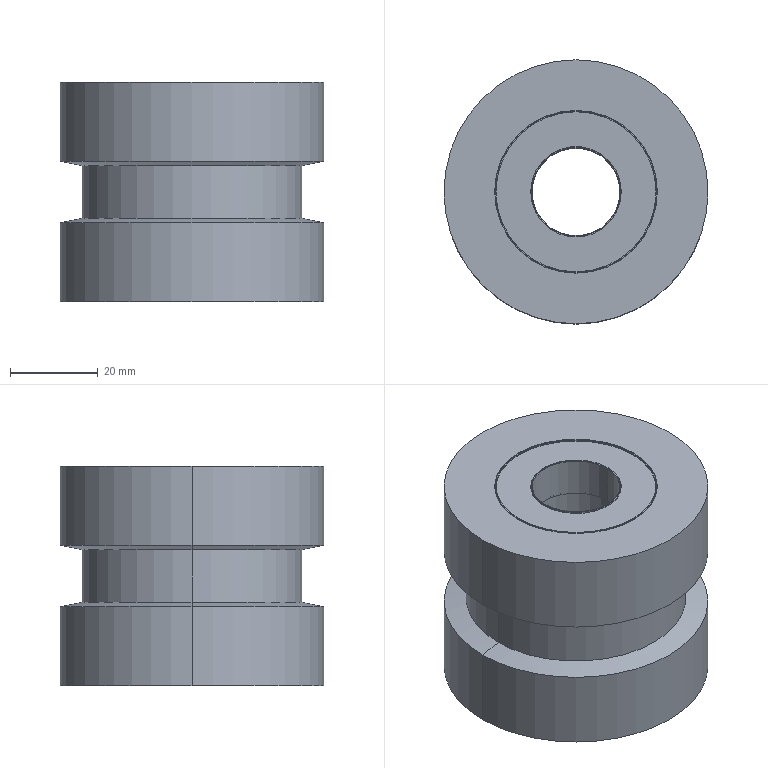Part | STEP file | ENJ11-D60-d20-L50-X14-Y12-Z5 flat belt idler Yihda 271 | 1 solid | 58 faces | box 60 x 60 x 50 mm | volume 111446 mm3 | cylinder 32 | plane 14 | torus 8 | cone 4 | commonest cylinder face diameters 20.6 x8 36.4 x8 20 x4 37 x4 60 x4 22 x2
STEP:
#1=CARTESIAN_POINT('',(10.3,0.,-41.));
#2=VERTEX_POINT('',#1);
#3=CARTESIAN_POINT('',(-10.3,0.,-41.));
#4=VERTEX_POINT('',#3);
#5=CARTESIAN_POINT('',(0.,0.,-41.));
#6=DIRECTION('',(0.,0.,-1.));
#7=DIRECTION('',(-1.,0.,0.));
#8=AXIS2_PLACEMENT_3D('',#5,#6,#7);
#9=CIRCLE('',#8,10.3);
#10=EDGE_CURVE('',#2,#4,#9,.T.);
#11=ORIENTED_EDGE('',*,*,#10,.T.);
#12=CARTESIAN_POINT('',(-10.3,0.,-41.3));
#13=VERTEX_POINT('',#12);
#14=CARTESIAN_POINT('',(-10.3,0.,-41.3));
#15=DIRECTION('',(0.,0.,1.));
#16=VECTOR('',#15,1000.);
#17=LINE('',#14,#16);
#18=EDGE_CURVE('',#13,#4,#17,.T.);
#19=ORIENTED_EDGE('',*,*,#18,.F.);
#20=CARTESIAN_POINT('',(10.3,0.,-41.3));
#21=VERTEX_POINT('',#20);
#22=CARTESIAN_POINT('',(0.,0.,-41.3));
#23=DIRECTION('',(0.,0.,-1.));
#24=DIRECTION('',(-1.,0.,0.));
#25=AXIS2_PLACEMENT_3D('',#22,#23,#24);
#26=CIRCLE('',#25,10.3);
#27=EDGE_CURVE('',#21,#13,#26,.T.);
#28=ORIENTED_EDGE('',*,*,#27,.F.);
#29=CARTESIAN_POINT('',(10.3,0.,-41.3));
#30=DIRECTION('',(0.,0.,1.));
#31=VECTOR('',#30,1000.);
#32=LINE('',#29,#31);
#33=EDGE_CURVE('',#21,#2,#32,.T.);
#34=ORIENTED_EDGE('',*,*,#33,.T.);
#35=EDGE_LOOP('',(#11,#19,#28,#34));
#36=FACE_OUTER_BOUND('',#35,.T.);
#37=CARTESIAN_POINT('',(0.,0.,-50.));
#38=DIRECTION('',(0.,0.,1.));
#39=DIRECTION('',(0.,1.,0.));
#40=AXIS2_PLACEMENT_3D('',#37,#38,#39);
#41=CYLINDRICAL_SURFACE('',#40,10.3);
#42=ADVANCED_FACE('',(#36),#41,.T.);
#43=CARTESIAN_POINT('',(0.,0.,-41.3));
#44=DIRECTION('',(0.,0.,-1.));
#45=DIRECTION('',(-1.,0.,0.));
#46=AXIS2_PLACEMENT_3D('',#43,#44,#45);
#47=CIRCLE('',#46,10.3);
#48=EDGE_CURVE('',#13,#21,#47,.T.);
#49=ORIENTED_EDGE('',*,*,#48,.F.);
#50=ORIENTED_EDGE('',*,*,#18,.T.);
#51=CARTESIAN_POINT('',(0.,0.,-41.));
#52=DIRECTION('',(0.,0.,-1.));
#53=DIRECTION('',(-1.,0.,0.));
#54=AXIS2_PLACEMENT_3D('',#51,#52,#53);
#55=CIRCLE('',#54,10.3);
#56=EDGE_CURVE('',#4,#2,#55,.T.);
#57=ORIENTED_EDGE('',*,*,#56,.T.);
#58=ORIENTED_EDGE('',*,*,#33,.F.);
#59=EDGE_LOOP('',(#49,#50,#57,#58));
#60=FACE_OUTER_BOUND('',#59,.T.);
#61=CARTESIAN_POINT('',(0.,0.,-50.));
#62=DIRECTION('',(0.,0.,1.));
#63=DIRECTION('',(0.,-1.,0.));
#64=AXIS2_PLACEMENT_3D('',#61,#62,#63);
#65=CYLINDRICAL_SURFACE('',#64,10.3);
#66=ADVANCED_FACE('',(#60),#65,.T.);
#67=CARTESIAN_POINT('',(-10.,0.,-41.));
#68=VERTEX_POINT('',#67);
#69=CARTESIAN_POINT('',(10.,0.,-41.));
#70=VERTEX_POINT('',#69);
#71=CARTESIAN_POINT('',(0.,0.,-41.));
#72=DIRECTION('',(0.,0.,-1.));
#73=DIRECTION('',(-1.,0.,0.));
#74=AXIS2_PLACEMENT_3D('',#71,#72,#73);
#75=CIRCLE('',#74,10.);
#76=EDGE_CURVE('',#68,#70,#75,.T.);
#77=ORIENTED_EDGE('',*,*,#76,.T.);
#78=CARTESIAN_POINT('',(0.,0.,-41.));
#79=DIRECTION('',(0.,0.,-1.));
#80=DIRECTION('',(-1.,0.,0.));
#81=AXIS2_PLACEMENT_3D('',#78,#79,#80);
#82=CIRCLE('',#81,10.);
#83=EDGE_CURVE('',#70,#68,#82,.T.);
#84=ORIENTED_EDGE('',*,*,#83,.T.);
#85=EDGE_LOOP('',(#77,#84));
#86=FACE_BOUND('',#85,.T.);
#87=ORIENTED_EDGE('',*,*,#56,.F.);
#88=ORIENTED_EDGE('',*,*,#10,.F.);
#89=EDGE_LOOP('',(#87,#88));
#90=FACE_OUTER_BOUND('',#89,.T.);
#91=CARTESIAN_POINT('',(0.,10.3,-41.));
#92=DIRECTION('',(0.,0.,1.));
#93=DIRECTION('',(1.,0.,0.));
#94=AXIS2_PLACEMENT_3D('',#91,#92,#93);
#95=PLANE('',#94);
#96=ADVANCED_FACE('',(#86,#90),#95,.T.);
#97=ORIENTED_EDGE('',*,*,#83,.F.);
#98=CARTESIAN_POINT('',(10.,0.,-49.9));
#99=VERTEX_POINT('',#98);
#100=CARTESIAN_POINT('',(10.,0.,-49.9));
#101=DIRECTION('',(0.,0.,1.));
#102=VECTOR('',#101,1000.);
#103=LINE('',#100,#102);
#104=EDGE_CURVE('',#99,#70,#103,.T.);
#105=ORIENTED_EDGE('',*,*,#104,.F.);
#106=CARTESIAN_POINT('',(-10.,0.,-49.9));
#107=VERTEX_POINT('',#106);
#108=CARTESIAN_POINT('',(0.,0.,-49.9));
#109=DIRECTION('',(0.,0.,-1.));
#110=DIRECTION('',(-1.,0.,0.));
#111=AXIS2_PLACEMENT_3D('',#108,#109,#110);
#112=CIRCLE('',#111,10.);
#113=EDGE_CURVE('',#99,#107,#112,.T.);
#114=ORIENTED_EDGE('',*,*,#113,.T.);
#115=CARTESIAN_POINT('',(-10.,0.,-49.9));
#116=DIRECTION('',(0.,0.,1.));
#117=VECTOR('',#116,1000.);
#118=LINE('',#115,#117);
#119=EDGE_CURVE('',#107,#68,#118,.T.);
#120=ORIENTED_EDGE('',*,*,#119,.T.);
#121=EDGE_LOOP('',(#97,#105,#114,#120));
#122=FACE_OUTER_BOUND('',#121,.T.);
#123=CARTESIAN_POINT('',(0.,0.,-50.));
#124=DIRECTION('',(0.,0.,1.));
#125=DIRECTION('',(0.,1.,0.));
#126=AXIS2_PLACEMENT_3D('',#123,#124,#125);
#127=CYLINDRICAL_SURFACE('',#126,10.);
#128=ADVANCED_FACE('',(#122),#127,.F.);
#129=CARTESIAN_POINT('',(0.,0.,-49.9));
#130=DIRECTION('',(0.,0.,-1.));
#131=DIRECTION('',(-1.,0.,0.));
#132=AXIS2_PLACEMENT_3D('',#129,#130,#131);
#133=CIRCLE('',#132,10.);
#134=EDGE_CURVE('',#107,#99,#133,.T.);
#135=ORIENTED_EDGE('',*,*,#134,.T.);
#136=ORIENTED_EDGE('',*,*,#104,.T.);
#137=ORIENTED_EDGE('',*,*,#76,.F.);
#138=ORIENTED_EDGE('',*,*,#119,.F.);
#139=EDGE_LOOP('',(#135,#136,#137,#138));
#140=FACE_OUTER_BOUND('',#139,.T.);
#141=CARTESIAN_POINT('',(0.,0.,-50.));
#142=DIRECTION('',(0.,0.,1.));
#143=DIRECTION('',(0.,-1.,0.));
#144=AXIS2_PLACEMENT_3D('',#141,#142,#143);
#145=CYLINDRICAL_SURFACE('',#144,10.);
#146=ADVANCED_FACE('',(#140),#145,.F.);
#147=ORIENTED_EDGE('',*,*,#134,.F.);
#148=CARTESIAN_POINT('',(-10.1,0.,-50.));
#149=VERTEX_POINT('',#148);
#150=CARTESIAN_POINT('',(-10.1,0.,-50.));
#151=CARTESIAN_POINT('',(-10.074,0.,-50.));
#152=CARTESIAN_POINT('',(-10.048,0.,-49.989));
#153=CARTESIAN_POINT('',(-10.011,0.,-49.952));
#154=CARTESIAN_POINT('',(-10.,0.,-49.926));
#155=CARTESIAN_POINT('',(-10.,0.,-49.9));
#156=B_SPLINE_CURVE_WITH_KNOTS('',3,(#150,#151,#152,#153,#154,#155),.UNSPECIFIED.,.F.,.F.,(4,2,4),(0.,0.7854,1.571),.UNSPECIFIED.);
#157=EDGE_CURVE('',#149,#107,#156,.T.);
#158=ORIENTED_EDGE('',*,*,#157,.F.);
#159=CARTESIAN_POINT('',(10.1,0.,-50.));
#160=VERTEX_POINT('',#159);
#161=CARTESIAN_POINT('',(0.,0.,-50.));
#162=DIRECTION('',(0.,0.,-1.));
#163=DIRECTION('',(-1.,0.,0.));
#164=AXIS2_PLACEMENT_3D('',#161,#162,#163);
#165=CIRCLE('',#164,10.1);
#166=EDGE_CURVE('',#149,#160,#165,.T.);
#167=ORIENTED_EDGE('',*,*,#166,.T.);
#168=CARTESIAN_POINT('',(10.1,0.,-50.));
#169=CARTESIAN_POINT('',(10.074,0.,-50.));
#170=CARTESIAN_POINT('',(10.048,0.,-49.989));
#171=CARTESIAN_POINT('',(10.011,0.,-49.952));
#172=CARTESIAN_POINT('',(10.,0.,-49.926));
#173=CARTESIAN_POINT('',(10.,0.,-49.9));
#174=B_SPLINE_CURVE_WITH_KNOTS('',3,(#168,#169,#170,#171,#172,#173),.UNSPECIFIED.,.F.,.F.,(4,2,4),(0.,0.7854,1.571),.UNSPECIFIED.);
#175=EDGE_CURVE('',#160,#99,#174,.T.);
#176=ORIENTED_EDGE('',*,*,#175,.T.);
#177=EDGE_LOOP('',(#147,#158,#167,#176));
#178=FACE_OUTER_BOUND('',#177,.T.);
#179=CARTESIAN_POINT('',(0.,0.,-49.9));
#180=DIRECTION('',(0.,0.,-1.));
#181=DIRECTION('',(0.,-1.,0.));
#182=AXIS2_PLACEMENT_3D('',#179,#180,#181);
#183=TOROIDAL_SURFACE('',#182,10.1,0.1);
#184=ADVANCED_FACE('',(#178),#183,.T.);
#185=CARTESIAN_POINT('',(0.,0.,-50.));
#186=DIRECTION('',(0.,0.,-1.));
#187=DIRECTION('',(-1.,0.,0.));
#188=AXIS2_PLACEMENT_3D('',#185,#186,#187);
#189=CIRCLE('',#188,10.1);
#190=EDGE_CURVE('',#160,#149,#189,.T.);
#191=ORIENTED_EDGE('',*,*,#190,.T.);
#192=ORIENTED_EDGE('',*,*,#157,.T.);
#193=ORIENTED_EDGE('',*,*,#113,.F.);
#194=ORIENTED_EDGE('',*,*,#175,.F.);
#195=EDGE_LOOP('',(#191,#192,#193,#194));
#196=FACE_OUTER_BOUND('',#195,.T.);
#197=CARTESIAN_POINT('',(0.,0.,-49.9));
#198=DIRECTION('',(0.,0.,-1.));
#199=DIRECTION('',(0.,1.,0.));
#200=AXIS2_PLACEMENT_3D('',#197,#198,#199);
#201=TOROIDAL_SURFACE('',#200,10.1,0.1);
#202=ADVANCED_FACE('',(#196),#201,.T.);
#203=CARTESIAN_POINT('',(-10.3,0.,-50.));
#204=VERTEX_POINT('',#203);
#205=CARTESIAN_POINT('',(10.3,0.,-50.));
#206=VERTEX_POINT('',#205);
#207=CARTESIAN_POINT('',(0.,0.,-50.));
#208=DIRECTION('',(0.,0.,-1.));
#209=DIRECTION('',(-1.,0.,0.));
#210=AXIS2_PLACEMENT_3D('',#207,#208,#209);
#211=CIRCLE('',#210,10.3);
#212=EDGE_CURVE('',#204,#206,#211,.T.);
#213=ORIENTED_EDGE('',*,*,#212,.T.);
#214=CARTESIAN_POINT('',(0.,0.,-50.));
#215=DIRECTION('',(0.,0.,-1.));
#216=DIRECTION('',(-1.,0.,0.));
#217=AXIS2_PLACEMENT_3D('',#214,#215,#216);
#218=CIRCLE('',#217,10.3);
#219=EDGE_CURVE('',#206,#204,#218,.T.);
#220=ORIENTED_EDGE('',*,*,#219,.T.);
#221=EDGE_LOOP('',(#213,#220));
#222=FACE_OUTER_BOUND('',#221,.T.);
#223=ORIENTED_EDGE('',*,*,#166,.F.);
#224=ORIENTED_EDGE('',*,*,#190,.F.);
#225=EDGE_LOOP('',(#223,#224));
#226=FACE_BOUND('',#225,.T.);
#227=CARTESIAN_POINT('',(0.,10.1,-50.));
#228=DIRECTION('',(0.,0.,-1.));
#229=DIRECTION('',(-1.,0.,0.));
#230=AXIS2_PLACEMENT_3D('',#227,#228,#229);
#231=PLANE('',#230);
#232=ADVANCED_FACE('',(#222,#226),#231,.T.);
#233=CARTESIAN_POINT('',(10.3,0.,-49.7));
#234=VERTEX_POINT('',#233);
#235=CARTESIAN_POINT('',(-10.3,0.,-49.7));
#236=VERTEX_POINT('',#235);
#237=CARTESIAN_POINT('',(0.,0.,-49.7));
#238=DIRECTION('',(0.,0.,-1.));
#239=DIRECTION('',(-1.,0.,0.));
#240=AXIS2_PLACEMENT_3D('',#237,#238,#239);
#241=CIRCLE('',#240,10.3);
#242=EDGE_CURVE('',#234,#236,#241,.T.);
#243=ORIENTED_EDGE('',*,*,#242,.T.);
#244=CARTESIAN_POINT('',(-10.3,0.,-50.));
#245=DIRECTION('',(0.,0.,1.));
#246=VECTOR('',#245,1000.);
#247=LINE('',#244,#246);
#248=EDGE_CURVE('',#204,#236,#247,.T.);
#249=ORIENTED_EDGE('',*,*,#248,.F.);
#250=ORIENTED_EDGE('',*,*,#219,.F.);
#251=CARTESIAN_POINT('',(10.3,0.,-50.));
#252=DIRECTION('',(0.,0.,1.));
#253=VECTOR('',#252,1000.);
#254=LINE('',#251,#253);
#255=EDGE_CURVE('',#206,#234,#254,.T.);
#256=ORIENTED_EDGE('',*,*,#255,.T.);
#257=EDGE_LOOP('',(#243,#249,#250,#256));
#258=FACE_OUTER_BOUND('',#257,.T.);
#259=CARTESIAN_POINT('',(0.,0.,-50.));
#260=DIRECTION('',(0.,0.,1.));
#261=DIRECTION('',(0.,1.,0.));
#262=AXIS2_PLACEMENT_3D('',#259,#260,#261);
#263=CYLINDRICAL_SURFACE('',#262,10.3);
#264=ADVANCED_FACE('',(#258),#263,.T.);
#265=ORIENTED_EDGE('',*,*,#212,.F.);
#266=ORIENTED_EDGE('',*,*,#248,.T.);
#267=CARTESIAN_POINT('',(0.,0.,-49.7));
#268=DIRECTION('',(0.,0.,-1.));
#269=DIRECTION('',(-1.,0.,0.));
#270=AXIS2_PLACEMENT_3D('',#267,#268,#269);
#271=CIRCLE('',#270,10.3);
#272=EDGE_CURVE('',#236,#234,#271,.T.);
#273=ORIENTED_EDGE('',*,*,#272,.T.);
#274=ORIENTED_EDGE('',*,*,#255,.F.);
#275=EDGE_LOOP('',(#265,#266,#273,#274));
#276=FACE_OUTER_BOUND('',#275,.T.);
#277=CARTESIAN_POINT('',(0.,0.,-50.));
#278=DIRECTION('',(0.,0.,1.));
#279=DIRECTION('',(0.,-1.,0.));
#280=AXIS2_PLACEMENT_3D('',#277,#278,#279);
#281=CYLINDRICAL_SURFACE('',#280,10.3);
#282=ADVANCED_FACE('',(#276),#281,.T.);
#283=CARTESIAN_POINT('',(-18.2,0.,-49.7));
#284=VERTEX_POINT('',#283);
#285=CARTESIAN_POINT('',(18.2,0.,-49.7));
#286=VERTEX_POINT('',#285);
#287=CARTESIAN_POINT('',(0.,0.,-49.7));
#288=DIRECTION('',(0.,0.,-1.));
#289=DIRECTION('',(-1.,0.,0.));
#290=AXIS2_PLACEMENT_3D('',#287,#288,#289);
#291=CIRCLE('',#290,18.2);
#292=EDGE_CURVE('',#284,#286,#291,.T.);
#293=ORIENTED_EDGE('',*,*,#292,.T.);
#294=CARTESIAN_POINT('',(0.,0.,-49.7));
#295=DIRECTION('',(0.,0.,-1.));
#296=DIRECTION('',(-1.,0.,0.));
#297=AXIS2_PLACEMENT_3D('',#294,#295,#296);
#298=CIRCLE('',#297,18.2);
#299=EDGE_CURVE('',#286,#284,#298,.T.);
#300=ORIENTED_EDGE('',*,*,#299,.T.);
#301=EDGE_LOOP('',(#293,#300));
#302=FACE_OUTER_BOUND('',#301,.T.);
#303=ORIENTED_EDGE('',*,*,#272,.F.);
#304=ORIENTED_EDGE('',*,*,#242,.F.);
#305=EDGE_LOOP('',(#303,#304));
#306=FACE_BOUND('',#305,.T.);
#307=CARTESIAN_POINT('',(0.,10.3,-49.7));
#308=DIRECTION('',(0.,0.,-1.));
#309=DIRECTION('',(-1.,0.,0.));
#310=AXIS2_PLACEMENT_3D('',#307,#308,#309);
#311=PLANE('',#310);
#312=ADVANCED_FACE('',(#302,#306),#311,.T.);
#313=ORIENTED_EDGE('',*,*,#299,.F.);
#314=CARTESIAN_POINT('',(18.2,0.,-50.));
#315=VERTEX_POINT('',#314);
#316=CARTESIAN_POINT('',(18.2,0.,-50.));
#317=DIRECTION('',(0.,0.,1.));
#318=VECTOR('',#317,1000.);
#319=LINE('',#316,#318);
#320=EDGE_CURVE('',#315,#286,#319,.T.);
#321=ORIENTED_EDGE('',*,*,#320,.F.);
#322=CARTESIAN_POINT('',(-18.2,0.,-50.));
#323=VERTEX_POINT('',#322);
#324=CARTESIAN_POINT('',(0.,0.,-50.));
#325=DIRECTION('',(0.,0.,-1.));
#326=DIRECTION('',(-1.,0.,0.));
#327=AXIS2_PLACEMENT_3D('',#324,#325,#326);
#328=CIRCLE('',#327,18.2);
#329=EDGE_CURVE('',#315,#323,#328,.T.);
#330=ORIENTED_EDGE('',*,*,#329,.T.);
#331=CARTESIAN_POINT('',(-18.2,0.,-50.));
#332=DIRECTION('',(0.,0.,1.));
#333=VECTOR('',#332,1000.);
#334=LINE('',#331,#333);
#335=EDGE_CURVE('',#323,#284,#334,.T.);
#336=ORIENTED_EDGE('',*,*,#335,.T.);
#337=EDGE_LOOP('',(#313,#321,#330,#336));
#338=FACE_OUTER_BOUND('',#337,.T.);
#339=CARTESIAN_POINT('',(0.,0.,-50.));
#340=DIRECTION('',(0.,0.,1.));
#341=DIRECTION('',(0.,1.,0.));
#342=AXIS2_PLACEMENT_3D('',#339,#340,#341);
#343=CYLINDRICAL_SURFACE('',#342,18.2);
#344=ADVANCED_FACE('',(#338),#343,.F.);
#345=CARTESIAN_POINT('',(0.,0.,-50.));
#346=DIRECTION('',(0.,0.,-1.));
#347=DIRECTION('',(-1.,0.,0.));
#348=AXIS2_PLACEMENT_3D('',#345,#346,#347);
#349=CIRCLE('',#348,18.2);
#350=EDGE_CURVE('',#323,#315,#349,.T.);
#351=ORIENTED_EDGE('',*,*,#350,.T.);
#352=ORIENTED_EDGE('',*,*,#320,.T.);
#353=ORIENTED_EDGE('',*,*,#292,.F.);
#354=ORIENTED_EDGE('',*,*,#335,.F.);
#355=EDGE_LOOP('',(#351,#352,#353,#354));
#356=FACE_OUTER_BOUND('',#355,.T.);
#357=CARTESIAN_POINT('',(0.,0.,-50.));
#358=DIRECTION('',(0.,0.,1.));
#359=DIRECTION('',(0.,-1.,0.));
#360=AXIS2_PLACEMENT_3D('',#357,#358,#359);
#361=CYLINDRICAL_SURFACE('',#360,18.2);
#362=ADVANCED_FACE('',(#356),#361,.F.);
#363=CARTESIAN_POINT('',(-18.4,0.,-50.));
#364=VERTEX_POINT('',#363);
#365=CARTESIAN_POINT('',(18.4,0.,-50.));
#366=VERTEX_POINT('',#365);
#367=CARTESIAN_POINT('',(0.,0.,-50.));
#368=DIRECTION('',(0.,0.,-1.));
#369=DIRECTION('',(-1.,0.,0.));
#370=AXIS2_PLACEMENT_3D('',#367,#368,#369);
#371=CIRCLE('',#370,18.4);
#372=EDGE_CURVE('',#364,#366,#371,.T.);
#373=ORIENTED_EDGE('',*,*,#372,.T.);
#374=CARTESIAN_POINT('',(0.,0.,-50.));
#375=DIRECTION('',(0.,0.,-1.));
#376=DIRECTION('',(-1.,0.,0.));
#377=AXIS2_PLACEMENT_3D('',#374,#375,#376);
#378=CIRCLE('',#377,18.4);
#379=EDGE_CURVE('',#366,#364,#378,.T.);
#380=ORIENTED_EDGE('',*,*,#379,.T.);
#381=EDGE_LOOP('',(#373,#380));
#382=FACE_OUTER_BOUND('',#381,.T.);
#383=ORIENTED_EDGE('',*,*,#350,.F.);
#384=ORIENTED_EDGE('',*,*,#329,.F.);
#385=EDGE_LOOP('',(#383,#384));
#386=FACE_BOUND('',#385,.T.);
#387=CARTESIAN_POINT('',(0.,18.2,-50.));
#388=DIRECTION('',(0.,0.,-1.));
#389=DIRECTION('',(-1.,0.,0.));
#390=AXIS2_PLACEMENT_3D('',#387,#388,#389);
#391=PLANE('',#390);
#392=ADVANCED_FACE('',(#382,#386),#391,.T.);
#393=CARTESIAN_POINT('',(18.5,0.,-49.9));
#394=VERTEX_POINT('',#393);
#395=CARTESIAN_POINT('',(-18.5,0.,-49.9));
#396=VERTEX_POINT('',#395);
#397=CARTESIAN_POINT('',(0.,0.,-49.9));
#398=DIRECTION('',(0.,0.,-1.));
#399=DIRECTION('',(-1.,0.,0.));
#400=AXIS2_PLACEMENT_3D('',#397,#398,#399);
#401=CIRCLE('',#400,18.5);
#402=EDGE_CURVE('',#394,#396,#401,.T.);
#403=ORIENTED_EDGE('',*,*,#402,.T.);
#404=CARTESIAN_POINT('',(-18.5,0.,-49.9));
#405=CARTESIAN_POINT('',(-18.5,0.,-49.926));
#406=CARTESIAN_POINT('',(-18.489,0.,-49.952));
#407=CARTESIAN_POINT('',(-18.452,0.,-49.989));
#408=CARTESIAN_POINT('',(-18.426,0.,-50.));
#409=CARTESIAN_POINT('',(-18.4,0.,-50.));
#410=B_SPLINE_CURVE_WITH_KNOTS('',3,(#404,#405,#406,#407,#408,#409),.UNSPECIFIED.,.F.,.F.,(4,2,4),(0.,0.7854,1.571),.UNSPECIFIED.);
#411=EDGE_CURVE('',#396,#364,#410,.T.);
#412=ORIENTED_EDGE('',*,*,#411,.T.);
#413=ORIENTED_EDGE('',*,*,#379,.F.);
#414=CARTESIAN_POINT('',(18.5,0.,-49.9));
#415=CARTESIAN_POINT('',(18.5,0.,-49.926));
#416=CARTESIAN_POINT('',(18.489,0.,-49.952));
#417=CARTESIAN_POINT('',(18.452,0.,-49.989));
#418=CARTESIAN_POINT('',(18.426,0.,-50.));
#419=CARTESIAN_POINT('',(18.4,0.,-50.));
#420=B_SPLINE_CURVE_WITH_KNOTS('',3,(#414,#415,#416,#417,#418,#419),.UNSPECIFIED.,.F.,.F.,(4,2,4),(0.,0.7854,1.571),.UNSPECIFIED.);
#421=EDGE_CURVE('',#394,#366,#420,.T.);
#422=ORIENTED_EDGE('',*,*,#421,.F.);
#423=EDGE_LOOP('',(#403,#412,#413,#422));
#424=FACE_OUTER_BOUND('',#423,.T.);
#425=CARTESIAN_POINT('',(0.,0.,-49.9));
#426=DIRECTION('',(0.,0.,-1.));
#427=DIRECTION('',(0.,1.,0.));
#428=AXIS2_PLACEMENT_3D('',#425,#426,#427);
#429=TOROIDAL_SURFACE('',#428,18.4,0.1);
#430=ADVANCED_FACE('',(#424),#429,.T.);
#431=ORIENTED_EDGE('',*,*,#372,.F.);
#432=ORIENTED_EDGE('',*,*,#411,.F.);
#433=CARTESIAN_POINT('',(0.,0.,-49.9));
#434=DIRECTION('',(0.,0.,-1.));
#435=DIRECTION('',(-1.,0.,0.));
#436=AXIS2_PLACEMENT_3D('',#433,#434,#435);
#437=CIRCLE('',#436,18.5);
#438=EDGE_CURVE('',#396,#394,#437,.T.);
#439=ORIENTED_EDGE('',*,*,#438,.T.);
#440=ORIENTED_EDGE('',*,*,#421,.T.);
#441=EDGE_LOOP('',(#431,#432,#439,#440));
#442=FACE_OUTER_BOUND('',#441,.T.);
#443=CARTESIAN_POINT('',(0.,0.,-49.9));
#444=DIRECTION('',(0.,0.,-1.));
#445=DIRECTION('',(0.,-1.,0.));
#446=AXIS2_PLACEMENT_3D('',#443,#444,#445);
#447=TOROIDAL_SURFACE('',#446,18.4,0.1);
#448=ADVANCED_FACE('',(#442),#447,.T.);
#449=CARTESIAN_POINT('',(-18.5,0.,-50.));
#450=VERTEX_POINT('',#449);
#451=CARTESIAN_POINT('',(18.5,0.,-50.));
#452=VERTEX_POINT('',#451);
#453=CARTESIAN_POINT('',(0.,0.,-50.));
#454=DIRECTION('',(0.,0.,-1.));
#455=DIRECTION('',(-1.,0.,0.));
#456=AXIS2_PLACEMENT_3D('',#453,#454,#455);
#457=CIRCLE('',#456,18.5);
#458=EDGE_CURVE('',#450,#452,#457,.T.);
#459=ORIENTED_EDGE('',*,*,#458,.T.);
#460=CARTESIAN_POINT('',(18.5,0.,-50.));
#461=DIRECTION('',(0.,0.,1.));
#462=VECTOR('',#461,1000.);
#463=LINE('',#460,#462);
#464=EDGE_CURVE('',#452,#394,#463,.T.);
#465=ORIENTED_EDGE('',*,*,#464,.T.);
#466=ORIENTED_EDGE('',*,*,#438,.F.);
#467=CARTESIAN_POINT('',(-18.5,0.,-50.));
#468=DIRECTION('',(0.,0.,1.));
#469=VECTOR('',#468,1000.);
#470=LINE('',#467,#469);
#471=EDGE_CURVE('',#450,#396,#470,.T.);
#472=ORIENTED_EDGE('',*,*,#471,.F.);
#473=EDGE_LOOP('',(#459,#465,#466,#472));
#474=FACE_OUTER_BOUND('',#473,.T.);
#475=CARTESIAN_POINT('',(0.,0.,-50.));
#476=DIRECTION('',(0.,0.,1.));
#477=DIRECTION('',(0.,-1.,0.));
#478=AXIS2_PLACEMENT_3D('',#475,#476,#477);
#479=CYLINDRICAL_SURFACE('',#478,18.5);
#480=ADVANCED_FACE('',(#474),#479,.F.);
#481=ORIENTED_EDGE('',*,*,#402,.F.);
#482=ORIENTED_EDGE('',*,*,#464,.F.);
#483=CARTESIAN_POINT('',(0.,0.,-50.));
#484=DIRECTION('',(0.,0.,-1.));
#485=DIRECTION('',(-1.,0.,0.));
#486=AXIS2_PLACEMENT_3D('',#483,#484,#485);
#487=CIRCLE('',#486,18.5);
#488=EDGE_CURVE('',#452,#450,#487,.T.);
#489=ORIENTED_EDGE('',*,*,#488,.T.);
#490=ORIENTED_EDGE('',*,*,#471,.T.);
#491=EDGE_LOOP('',(#481,#482,#489,#490));
#492=FACE_OUTER_BOUND('',#491,.T.);
#493=CARTESIAN_POINT('',(0.,0.,-50.));
#494=DIRECTION('',(0.,0.,1.));
#495=DIRECTION('',(0.,1.,0.));
#496=AXIS2_PLACEMENT_3D('',#493,#494,#495);
#497=CYLINDRICAL_SURFACE('',#496,18.5);
#498=ADVANCED_FACE('',(#492),#497,.F.);
#499=CARTESIAN_POINT('',(-30.,0.,-50.));
#500=VERTEX_POINT('',#499);
#501=CARTESIAN_POINT('',(30.,0.,-50.));
#502=VERTEX_POINT('',#501);
#503=CARTESIAN_POINT('',(0.,0.,-50.));
#504=DIRECTION('',(0.,0.,-1.));
#505=DIRECTION('',(-1.,0.,0.));
#506=AXIS2_PLACEMENT_3D('',#503,#504,#505);
#507=CIRCLE('',#506,30.);
#508=EDGE_CURVE('',#500,#502,#507,.T.);
#509=ORIENTED_EDGE('',*,*,#508,.T.);
#510=CARTESIAN_POINT('',(0.,0.,-50.));
#511=DIRECTION('',(0.,0.,-1.));
#512=DIRECTION('',(-1.,0.,0.));
#513=AXIS2_PLACEMENT_3D('',#510,#511,#512);
#514=CIRCLE('',#513,30.);
#515=EDGE_CURVE('',#502,#500,#514,.T.);
#516=ORIENTED_EDGE('',*,*,#515,.T.);
#517=EDGE_LOOP('',(#509,#516));
#518=FACE_OUTER_BOUND('',#517,.T.);
#519=ORIENTED_EDGE('',*,*,#458,.F.);
#520=ORIENTED_EDGE('',*,*,#488,.F.);
#521=EDGE_LOOP('',(#519,#520));
#522=FACE_BOUND('',#521,.T.);
#523=CARTESIAN_POINT('',(0.,18.5,-50.));
#524=DIRECTION('',(0.,0.,-1.));
#525=DIRECTION('',(-1.,0.,0.));
#526=AXIS2_PLACEMENT_3D('',#523,#524,#525);
#527=PLANE('',#526);
#528=ADVANCED_FACE('',(#518,#522),#527,.T.);
#529=CARTESIAN_POINT('',(30.,0.,-32.));
#530=VERTEX_POINT('',#529);
#531=CARTESIAN_POINT('',(-30.,0.,-32.));
#532=VERTEX_POINT('',#531);
#533=CARTESIAN_POINT('',(0.,0.,-32.));
#534=DIRECTION('',(0.,0.,-1.));
#535=DIRECTION('',(-1.,0.,0.));
#536=AXIS2_PLACEMENT_3D('',#533,#534,#535);
#537=CIRCLE('',#536,30.);
#538=EDGE_CURVE('',#530,#532,#537,.T.);
#539=ORIENTED_EDGE('',*,*,#538,.T.);
#540=CARTESIAN_POINT('',(-30.,0.,-50.));
#541=DIRECTION('',(0.,0.,1.));
#542=VECTOR('',#541,1000.);
#543=LINE('',#540,#542);
#544=EDGE_CURVE('',#500,#532,#543,.T.);
#545=ORIENTED_EDGE('',*,*,#544,.F.);
#546=ORIENTED_EDGE('',*,*,#515,.F.);
#547=CARTESIAN_POINT('',(30.,0.,-50.));
#548=DIRECTION('',(0.,0.,1.));
#549=VECTOR('',#548,1000.);
#550=LINE('',#547,#549);
#551=EDGE_CURVE('',#502,#530,#550,.T.);
#552=ORIENTED_EDGE('',*,*,#551,.T.);
#553=EDGE_LOOP('',(#539,#545,#546,#552));
#554=FACE_OUTER_BOUND('',#553,.T.);
#555=CARTESIAN_POINT('',(0.,0.,-50.));
#556=DIRECTION('',(0.,0.,1.));
#557=DIRECTION('',(0.,1.,0.));
#558=AXIS2_PLACEMENT_3D('',#555,#556,#557);
#559=CYLINDRICAL_SURFACE('',#558,30.);
#560=ADVANCED_FACE('',(#554),#559,.T.);
#561=ORIENTED_EDGE('',*,*,#508,.F.);
#562=ORIENTED_EDGE('',*,*,#544,.T.);
#563=CARTESIAN_POINT('',(0.,0.,-32.));
#564=DIRECTION('',(0.,0.,-1.));
#565=DIRECTION('',(-1.,0.,0.));
#566=AXIS2_PLACEMENT_3D('',#563,#564,#565);
#567=CIRCLE('',#566,30.);
#568=EDGE_CURVE('',#532,#530,#567,.T.);
#569=ORIENTED_EDGE('',*,*,#568,.T.);
#570=ORIENTED_EDGE('',*,*,#551,.F.);
#571=EDGE_LOOP('',(#561,#562,#569,#570));
#572=FACE_OUTER_BOUND('',#571,.T.);
#573=CARTESIAN_POINT('',(0.,0.,-50.));
#574=DIRECTION('',(0.,0.,1.));
#575=DIRECTION('',(0.,-1.,0.));
#576=AXIS2_PLACEMENT_3D('',#573,#574,#575);
#577=CYLINDRICAL_SURFACE('',#576,30.);
#578=ADVANCED_FACE('',(#572),#577,.T.);
#579=ORIENTED_EDGE('',*,*,#568,.F.);
#580=CARTESIAN_POINT('',(-25.,0.,-31.));
#581=VERTEX_POINT('',#580);
#582=CARTESIAN_POINT('',(-25.,0.,-31.));
#583=DIRECTION('',(-0.9806,0.,-0.1961));
#584=VECTOR('',#583,1000.);
#585=LINE('',#582,#584);
#586=EDGE_CURVE('',#581,#532,#585,.T.);
#587=ORIENTED_EDGE('',*,*,#586,.F.);
#588=CARTESIAN_POINT('',(25.,0.,-31.));
#589=VERTEX_POINT('',#588);
#590=CARTESIAN_POINT('',(0.,0.,-31.));
#591=DIRECTION('',(0.,0.,-1.));
#592=DIRECTION('',(-1.,0.,0.));
#593=AXIS2_PLACEMENT_3D('',#590,#591,#592);
#594=CIRCLE('',#593,25.);
#595=EDGE_CURVE('',#581,#589,#594,.T.);
#596=ORIENTED_EDGE('',*,*,#595,.T.);
#597=CARTESIAN_POINT('',(25.,0.,-31.));
#598=DIRECTION('',(0.9806,0.,-0.1961));
#599=VECTOR('',#598,1000.);
#600=LINE('',#597,#599);
#601=EDGE_CURVE('',#589,#530,#600,.T.);
#602=ORIENTED_EDGE('',*,*,#601,.T.);
#603=EDGE_LOOP('',(#579,#587,#596,#602));
#604=FACE_OUTER_BOUND('',#603,.T.);
#605=CARTESIAN_POINT('',(0.,0.,-31.));
#606=DIRECTION('',(0.,0.,-1.));
#607=DIRECTION('',(0.,-1.,0.));
#608=AXIS2_PLACEMENT_3D('',#605,#606,#607);
#609=CONICAL_SURFACE('',#608,25.,1.373);
#610=ADVANCED_FACE('',(#604),#609,.T.);
#611=CARTESIAN_POINT('',(0.,0.,-31.));
#612=DIRECTION('',(0.,0.,-1.));
#613=DIRECTION('',(-1.,0.,0.));
#614=AXIS2_PLACEMENT_3D('',#611,#612,#613);
#615=CIRCLE('',#614,25.);
#616=EDGE_CURVE('',#589,#581,#615,.T.);
#617=ORIENTED_EDGE('',*,*,#616,.T.);
#618=ORIENTED_EDGE('',*,*,#586,.T.);
#619=ORIENTED_EDGE('',*,*,#538,.F.);
#620=ORIENTED_EDGE('',*,*,#601,.F.);
#621=EDGE_LOOP('',(#617,#618,#619,#620));
#622=FACE_OUTER_BOUND('',#621,.T.);
#623=CARTESIAN_POINT('',(0.,0.,-31.));
#624=DIRECTION('',(0.,0.,-1.));
#625=DIRECTION('',(0.,1.,0.));
#626=AXIS2_PLACEMENT_3D('',#623,#624,#625);
#627=CONICAL_SURFACE('',#626,25.,1.373);
#628=ADVANCED_FACE('',(#622),#627,.T.);
#629=CARTESIAN_POINT('',(25.,0.,-19.));
#630=VERTEX_POINT('',#629);
#631=CARTESIAN_POINT('',(-25.,0.,-19.));
#632=VERTEX_POINT('',#631);
#633=CARTESIAN_POINT('',(0.,0.,-19.));
#634=DIRECTION('',(0.,0.,-1.));
#635=DIRECTION('',(-1.,0.,0.));
#636=AXIS2_PLACEMENT_3D('',#633,#634,#635);
#637=CIRCLE('',#636,25.);
#638=EDGE_CURVE('',#630,#632,#637,.T.);
#639=ORIENTED_EDGE('',*,*,#638,.T.);
#640=CARTESIAN_POINT('',(-25.,0.,-31.));
#641=DIRECTION('',(0.,0.,1.));
#642=VECTOR('',#641,1000.);
#643=LINE('',#640,#642);
#644=EDGE_CURVE('',#581,#632,#643,.T.);
#645=ORIENTED_EDGE('',*,*,#644,.F.);
#646=ORIENTED_EDGE('',*,*,#616,.F.);
#647=CARTESIAN_POINT('',(25.,0.,-31.));
#648=DIRECTION('',(0.,0.,1.));
#649=VECTOR('',#648,1000.);
#650=LINE('',#647,#649);
#651=EDGE_CURVE('',#589,#630,#650,.T.);
#652=ORIENTED_EDGE('',*,*,#651,.T.);
#653=EDGE_LOOP('',(#639,#645,#646,#652));
#654=FACE_OUTER_BOUND('',#653,.T.);
#655=CARTESIAN_POINT('',(0.,0.,-50.));
#656=DIRECTION('',(0.,0.,1.));
#657=DIRECTION('',(0.,1.,0.));
#658=AXIS2_PLACEMENT_3D('',#655,#656,#657);
#659=CYLINDRICAL_SURFACE('',#658,25.);
#660=ADVANCED_FACE('',(#654),#659,.T.);
#661=ORIENTED_EDGE('',*,*,#595,.F.);
#662=ORIENTED_EDGE('',*,*,#644,.T.);
#663=CARTESIAN_POINT('',(0.,0.,-19.));
#664=DIRECTION('',(0.,0.,-1.));
#665=DIRECTION('',(-1.,0.,0.));
#666=AXIS2_PLACEMENT_3D('',#663,#664,#665);
#667=CIRCLE('',#666,25.);
#668=EDGE_CURVE('',#632,#630,#667,.T.);
#669=ORIENTED_EDGE('',*,*,#668,.T.);
#670=ORIENTED_EDGE('',*,*,#651,.F.);
#671=EDGE_LOOP('',(#661,#662,#669,#670));
#672=FACE_OUTER_BOUND('',#671,.T.);
#673=CARTESIAN_POINT('',(0.,0.,-50.));
#674=DIRECTION('',(0.,0.,1.));
#675=DIRECTION('',(0.,-1.,0.));
#676=AXIS2_PLACEMENT_3D('',#673,#674,#675);
#677=CYLINDRICAL_SURFACE('',#676,25.);
#678=ADVANCED_FACE('',(#672),#677,.T.);
#679=ORIENTED_EDGE('',*,*,#668,.F.);
#680=CARTESIAN_POINT('',(-30.,0.,-18.));
#681=VERTEX_POINT('',#680);
#682=CARTESIAN_POINT('',(-25.,0.,-19.));
#683=DIRECTION('',(-0.9806,0.,0.1961));
#684=VECTOR('',#683,1000.);
#685=LINE('',#682,#684);
#686=EDGE_CURVE('',#632,#681,#685,.T.);
#687=ORIENTED_EDGE('',*,*,#686,.T.);
#688=CARTESIAN_POINT('',(30.,0.,-18.));
#689=VERTEX_POINT('',#688);
#690=CARTESIAN_POINT('',(0.,0.,-18.));
#691=DIRECTION('',(0.,0.,-1.));
#692=DIRECTION('',(-1.,0.,0.));
#693=AXIS2_PLACEMENT_3D('',#690,#691,#692);
#694=CIRCLE('',#693,30.);
#695=EDGE_CURVE('',#681,#689,#694,.T.);
#696=ORIENTED_EDGE('',*,*,#695,.T.);
#697=CARTESIAN_POINT('',(25.,0.,-19.));
#698=DIRECTION('',(0.9806,0.,0.1961));
#699=VECTOR('',#698,1000.);
#700=LINE('',#697,#699);
#701=EDGE_CURVE('',#630,#689,#700,.T.);
#702=ORIENTED_EDGE('',*,*,#701,.F.);
#703=EDGE_LOOP('',(#679,#687,#696,#702));
#704=FACE_OUTER_BOUND('',#703,.T.);
#705=CARTESIAN_POINT('',(0.,0.,-18.));
#706=DIRECTION('',(0.,0.,1.));
#707=DIRECTION('',(0.,-1.,0.));
#708=AXIS2_PLACEMENT_3D('',#705,#706,#707);
#709=CONICAL_SURFACE('',#708,30.,1.373);
#710=ADVANCED_FACE('',(#704),#709,.T.);
#711=CARTESIAN_POINT('',(0.,0.,-18.));
#712=DIRECTION('',(0.,0.,-1.));
#713=DIRECTION('',(-1.,0.,0.));
#714=AXIS2_PLACEMENT_3D('',#711,#712,#713);
#715=CIRCLE('',#714,30.);
#716=EDGE_CURVE('',#689,#681,#715,.T.);
#717=ORIENTED_EDGE('',*,*,#716,.T.);
#718=ORIENTED_EDGE('',*,*,#686,.F.);
#719=ORIENTED_EDGE('',*,*,#638,.F.);
#720=ORIENTED_EDGE('',*,*,#701,.T.);
#721=EDGE_LOOP('',(#717,#718,#719,#720));
#722=FACE_OUTER_BOUND('',#721,.T.);
#723=CARTESIAN_POINT('',(0.,0.,-18.));
#724=DIRECTION('',(0.,0.,1.));
#725=DIRECTION('',(0.,1.,0.));
#726=AXIS2_PLACEMENT_3D('',#723,#724,#725);
#727=CONICAL_SURFACE('',#726,30.,1.373);
#728=ADVANCED_FACE('',(#722),#727,.T.);
#729=CARTESIAN_POINT('',(30.,0.,0.));
#730=VERTEX_POINT('',#729);
#731=CARTESIAN_POINT('',(-30.,0.,0.));
#732=VERTEX_POINT('',#731);
#733=CARTESIAN_POINT('',(0.,0.,0.));
#734=DIRECTION('',(0.,0.,-1.));
#735=DIRECTION('',(-1.,0.,0.));
#736=AXIS2_PLACEMENT_3D('',#733,#734,#735);
#737=CIRCLE('',#736,30.);
#738=EDGE_CURVE('',#730,#732,#737,.T.);
#739=ORIENTED_EDGE('',*,*,#738,.T.);
#740=CARTESIAN_POINT('',(-30.,0.,-18.));
#741=DIRECTION('',(0.,0.,1.));
#742=VECTOR('',#741,1000.);
#743=LINE('',#740,#742);
#744=EDGE_CURVE('',#681,#732,#743,.T.);
#745=ORIENTED_EDGE('',*,*,#744,.F.);
#746=ORIENTED_EDGE('',*,*,#716,.F.);
#747=CARTESIAN_POINT('',(30.,0.,-18.));
#748=DIRECTION('',(0.,0.,1.));
#749=VECTOR('',#748,1000.);
#750=LINE('',#747,#749);
#751=EDGE_CURVE('',#689,#730,#750,.T.);
#752=ORIENTED_EDGE('',*,*,#751,.T.);
#753=EDGE_LOOP('',(#739,#745,#746,#752));
#754=FACE_OUTER_BOUND('',#753,.T.);
#755=CARTESIAN_POINT('',(0.,0.,-50.));
#756=DIRECTION('',(0.,0.,1.));
#757=DIRECTION('',(0.,1.,0.));
#758=AXIS2_PLACEMENT_3D('',#755,#756,#757);
#759=CYLINDRICAL_SURFACE('',#758,30.);
#760=ADVANCED_FACE('',(#754),#759,.T.);
#761=ORIENTED_EDGE('',*,*,#695,.F.);
#762=ORIENTED_EDGE('',*,*,#744,.T.);
#763=CARTESIAN_POINT('',(0.,0.,0.));
#764=DIRECTION('',(0.,0.,-1.));
#765=DIRECTION('',(-1.,0.,0.));
#766=AXIS2_PLACEMENT_3D('',#763,#764,#765);
#767=CIRCLE('',#766,30.);
#768=EDGE_CURVE('',#732,#730,#767,.T.);
#769=ORIENTED_EDGE('',*,*,#768,.T.);
#770=ORIENTED_EDGE('',*,*,#751,.F.);
#771=EDGE_LOOP('',(#761,#762,#769,#770));
#772=FACE_OUTER_BOUND('',#771,.T.);
#773=CARTESIAN_POINT('',(0.,0.,-50.));
#774=DIRECTION('',(0.,0.,1.));
#775=DIRECTION('',(0.,-1.,0.));
#776=AXIS2_PLACEMENT_3D('',#773,#774,#775);
#777=CYLINDRICAL_SURFACE('',#776,30.);
#778=ADVANCED_FACE('',(#772),#777,.T.);
#779=CARTESIAN_POINT('',(-18.5,0.,0.));
#780=VERTEX_POINT('',#779);
#781=CARTESIAN_POINT('',(18.5,0.,0.));
#782=VERTEX_POINT('',#781);
#783=CARTESIAN_POINT('',(0.,0.,0.));
#784=DIRECTION('',(0.,0.,-1.));
#785=DIRECTION('',(-1.,0.,0.));
#786=AXIS2_PLACEMENT_3D('',#783,#784,#785);
#787=CIRCLE('',#786,18.5);
#788=EDGE_CURVE('',#780,#782,#787,.T.);
#789=ORIENTED_EDGE('',*,*,#788,.T.);
#790=CARTESIAN_POINT('',(0.,0.,0.));
#791=DIRECTION('',(0.,0.,-1.));
#792=DIRECTION('',(-1.,0.,0.));
#793=AXIS2_PLACEMENT_3D('',#790,#791,#792);
#794=CIRCLE('',#793,18.5);
#795=EDGE_CURVE('',#782,#780,#794,.T.);
#796=ORIENTED_EDGE('',*,*,#795,.T.);
#797=EDGE_LOOP('',(#789,#796));
#798=FACE_BOUND('',#797,.T.);
#799=ORIENTED_EDGE('',*,*,#768,.F.);
#800=ORIENTED_EDGE('',*,*,#738,.F.);
#801=EDGE_LOOP('',(#799,#800));
#802=FACE_OUTER_BOUND('',#801,.T.);
#803=CARTESIAN_POINT('',(0.,30.,0.));
#804=DIRECTION('',(0.,0.,1.));
#805=DIRECTION('',(1.,0.,0.));
#806=AXIS2_PLACEMENT_3D('',#803,#804,#805);
#807=PLANE('',#806);
#808=ADVANCED_FACE('',(#798,#802),#807,.T.);
#809=ORIENTED_EDGE('',*,*,#795,.F.);
#810=CARTESIAN_POINT('',(18.5,0.,-0.1));
#811=VERTEX_POINT('',#810);
#812=CARTESIAN_POINT('',(18.5,0.,-0.1));
#813=DIRECTION('',(0.,0.,1.));
#814=VECTOR('',#813,1000.);
#815=LINE('',#812,#814);
#816=EDGE_CURVE('',#811,#782,#815,.T.);
#817=ORIENTED_EDGE('',*,*,#816,.F.);
#818=CARTESIAN_POINT('',(-18.5,0.,-0.1));
#819=VERTEX_POINT('',#818);
#820=CARTESIAN_POINT('',(0.,0.,-0.1));
#821=DIRECTION('',(0.,0.,-1.));
#822=DIRECTION('',(-1.,0.,0.));
#823=AXIS2_PLACEMENT_3D('',#820,#821,#822);
#824=CIRCLE('',#823,18.5);
#825=EDGE_CURVE('',#811,#819,#824,.T.);
#826=ORIENTED_EDGE('',*,*,#825,.T.);
#827=CARTESIAN_POINT('',(-18.5,0.,-0.1));
#828=DIRECTION('',(0.,0.,1.));
#829=VECTOR('',#828,1000.);
#830=LINE('',#827,#829);
#831=EDGE_CURVE('',#819,#780,#830,.T.);
#832=ORIENTED_EDGE('',*,*,#831,.T.);
#833=EDGE_LOOP('',(#809,#817,#826,#832));
#834=FACE_OUTER_BOUND('',#833,.T.);
#835=CARTESIAN_POINT('',(0.,0.,-50.));
#836=DIRECTION('',(0.,0.,1.));
#837=DIRECTION('',(0.,1.,0.));
#838=AXIS2_PLACEMENT_3D('',#835,#836,#837);
#839=CYLINDRICAL_SURFACE('',#838,18.5);
#840=ADVANCED_FACE('',(#834),#839,.F.);
#841=CARTESIAN_POINT('',(0.,0.,-0.1));
#842=DIRECTION('',(0.,0.,-1.));
#843=DIRECTION('',(-1.,0.,0.));
#844=AXIS2_PLACEMENT_3D('',#841,#842,#843);
#845=CIRCLE('',#844,18.5);
#846=EDGE_CURVE('',#819,#811,#845,.T.);
#847=ORIENTED_EDGE('',*,*,#846,.T.);
#848=ORIENTED_EDGE('',*,*,#816,.T.);
#849=ORIENTED_EDGE('',*,*,#788,.F.);
#850=ORIENTED_EDGE('',*,*,#831,.F.);
#851=EDGE_LOOP('',(#847,#848,#849,#850));
#852=FACE_OUTER_BOUND('',#851,.T.);
#853=CARTESIAN_POINT('',(0.,0.,-50.));
#854=DIRECTION('',(0.,0.,1.));
#855=DIRECTION('',(0.,-1.,0.));
#856=AXIS2_PLACEMENT_3D('',#853,#854,#855);
#857=CYLINDRICAL_SURFACE('',#856,18.5);
#858=ADVANCED_FACE('',(#852),#857,.F.);
#859=ORIENTED_EDGE('',*,*,#846,.F.);
#860=CARTESIAN_POINT('',(-18.4,0.,0.));
#861=VERTEX_POINT('',#860);
#862=CARTESIAN_POINT('',(-18.4,0.,0.));
#863=CARTESIAN_POINT('',(-18.426,0.,0.));
#864=CARTESIAN_POINT('',(-18.452,0.,-0.01078));
#865=CARTESIAN_POINT('',(-18.489,0.,-0.0478));
#866=CARTESIAN_POINT('',(-18.5,0.,-0.07382));
#867=CARTESIAN_POINT('',(-18.5,0.,-0.1));
#868=B_SPLINE_CURVE_WITH_KNOTS('',3,(#862,#863,#864,#865,#866,#867),.UNSPECIFIED.,.F.,.F.,(4,2,4),(0.,0.7854,1.571),.UNSPECIFIED.);
#869=EDGE_CURVE('',#861,#819,#868,.T.);
#870=ORIENTED_EDGE('',*,*,#869,.F.);
#871=CARTESIAN_POINT('',(18.4,0.,0.));
#872=VERTEX_POINT('',#871);
#873=CARTESIAN_POINT('',(0.,0.,0.));
#874=DIRECTION('',(0.,0.,-1.));
#875=DIRECTION('',(-1.,0.,0.));
#876=AXIS2_PLACEMENT_3D('',#873,#874,#875);
#877=CIRCLE('',#876,18.4);
#878=EDGE_CURVE('',#861,#872,#877,.T.);
#879=ORIENTED_EDGE('',*,*,#878,.T.);
#880=CARTESIAN_POINT('',(18.4,0.,0.));
#881=CARTESIAN_POINT('',(18.426,0.,0.));
#882=CARTESIAN_POINT('',(18.452,0.,-0.01078));
#883=CARTESIAN_POINT('',(18.489,0.,-0.0478));
#884=CARTESIAN_POINT('',(18.5,0.,-0.07382));
#885=CARTESIAN_POINT('',(18.5,0.,-0.1));
#886=B_SPLINE_CURVE_WITH_KNOTS('',3,(#880,#881,#882,#883,#884,#885),.UNSPECIFIED.,.F.,.F.,(4,2,4),(0.,0.7854,1.571),.UNSPECIFIED.);
#887=EDGE_CURVE('',#872,#811,#886,.T.);
#888=ORIENTED_EDGE('',*,*,#887,.T.);
#889=EDGE_LOOP('',(#859,#870,#879,#888));
#890=FACE_OUTER_BOUND('',#889,.T.);
#891=CARTESIAN_POINT('',(0.,0.,-0.1));
#892=DIRECTION('',(0.,0.,-1.));
#893=DIRECTION('',(0.,-1.,0.));
#894=AXIS2_PLACEMENT_3D('',#891,#892,#893);
#895=TOROIDAL_SURFACE('',#894,18.4,0.1);
#896=ADVANCED_FACE('',(#890),#895,.T.);
#897=CARTESIAN_POINT('',(0.,0.,0.));
#898=DIRECTION('',(0.,0.,-1.));
#899=DIRECTION('',(-1.,0.,0.));
#900=AXIS2_PLACEMENT_3D('',#897,#898,#899);
#901=CIRCLE('',#900,18.4);
#902=EDGE_CURVE('',#872,#861,#901,.T.);
#903=ORIENTED_EDGE('',*,*,#902,.T.);
#904=ORIENTED_EDGE('',*,*,#869,.T.);
#905=ORIENTED_EDGE('',*,*,#825,.F.);
#906=ORIENTED_EDGE('',*,*,#887,.F.);
#907=EDGE_LOOP('',(#903,#904,#905,#906));
#908=FACE_OUTER_BOUND('',#907,.T.);
#909=CARTESIAN_POINT('',(0.,0.,-0.1));
#910=DIRECTION('',(0.,0.,-1.));
#911=DIRECTION('',(0.,1.,0.));
#912=AXIS2_PLACEMENT_3D('',#909,#910,#911);
#913=TOROIDAL_SURFACE('',#912,18.4,0.1);
#914=ADVANCED_FACE('',(#908),#913,.T.);
#915=CARTESIAN_POINT('',(-18.2,0.,0.));
#916=VERTEX_POINT('',#915);
#917=CARTESIAN_POINT('',(18.2,0.,0.));
#918=VERTEX_POINT('',#917);
#919=CARTESIAN_POINT('',(0.,0.,0.));
#920=DIRECTION('',(0.,0.,-1.));
#921=DIRECTION('',(-1.,0.,0.));
#922=AXIS2_PLACEMENT_3D('',#919,#920,#921);
#923=CIRCLE('',#922,18.2);
#924=EDGE_CURVE('',#916,#918,#923,.T.);
#925=ORIENTED_EDGE('',*,*,#924,.T.);
#926=CARTESIAN_POINT('',(0.,0.,0.));
#927=DIRECTION('',(0.,0.,-1.));
#928=DIRECTION('',(-1.,0.,0.));
#929=AXIS2_PLACEMENT_3D('',#926,#927,#928);
#930=CIRCLE('',#929,18.2);
#931=EDGE_CURVE('',#918,#916,#930,.T.);
#932=ORIENTED_EDGE('',*,*,#931,.T.);
#933=EDGE_LOOP('',(#925,#932));
#934=FACE_BOUND('',#933,.T.);
#935=ORIENTED_EDGE('',*,*,#878,.F.);
#936=ORIENTED_EDGE('',*,*,#902,.F.);
#937=EDGE_LOOP('',(#935,#936));
#938=FACE_OUTER_BOUND('',#937,.T.);
#939=CARTESIAN_POINT('',(0.,18.4,0.));
#940=DIRECTION('',(0.,0.,1.));
#941=DIRECTION('',(1.,0.,0.));
#942=AXIS2_PLACEMENT_3D('',#939,#940,#941);
#943=PLANE('',#942);
#944=ADVANCED_FACE('',(#934,#938),#943,.T.);
#945=ORIENTED_EDGE('',*,*,#931,.F.);
#946=CARTESIAN_POINT('',(18.2,0.,-0.3));
#947=VERTEX_POINT('',#946);
#948=CARTESIAN_POINT('',(18.2,0.,-0.3));
#949=DIRECTION('',(0.,0.,1.));
#950=VECTOR('',#949,1000.);
#951=LINE('',#948,#950);
#952=EDGE_CURVE('',#947,#918,#951,.T.);
#953=ORIENTED_EDGE('',*,*,#952,.F.);
#954=CARTESIAN_POINT('',(-18.2,0.,-0.3));
#955=VERTEX_POINT('',#954);
#956=CARTESIAN_POINT('',(0.,0.,-0.3));
#957=DIRECTION('',(0.,0.,-1.));
#958=DIRECTION('',(-1.,0.,0.));
#959=AXIS2_PLACEMENT_3D('',#956,#957,#958);
#960=CIRCLE('',#959,18.2);
#961=EDGE_CURVE('',#947,#955,#960,.T.);
#962=ORIENTED_EDGE('',*,*,#961,.T.);
#963=CARTESIAN_POINT('',(-18.2,0.,-0.3));
#964=DIRECTION('',(0.,0.,1.));
#965=VECTOR('',#964,1000.);
#966=LINE('',#963,#965);
#967=EDGE_CURVE('',#955,#916,#966,.T.);
#968=ORIENTED_EDGE('',*,*,#967,.T.);
#969=EDGE_LOOP('',(#945,#953,#962,#968));
#970=FACE_OUTER_BOUND('',#969,.T.);
#971=CARTESIAN_POINT('',(0.,0.,-9.));
#972=DIRECTION('',(0.,0.,1.));
#973=DIRECTION('',(0.,1.,0.));
#974=AXIS2_PLACEMENT_3D('',#971,#972,#973);
#975=CYLINDRICAL_SURFACE('',#974,18.2);
#976=ADVANCED_FACE('',(#970),#975,.F.);
#977=CARTESIAN_POINT('',(0.,0.,-0.3));
#978=DIRECTION('',(0.,0.,-1.));
#979=DIRECTION('',(-1.,0.,0.));
#980=AXIS2_PLACEMENT_3D('',#977,#978,#979);
#981=CIRCLE('',#980,18.2);
#982=EDGE_CURVE('',#955,#947,#981,.T.);
#983=ORIENTED_EDGE('',*,*,#982,.T.);
#984=ORIENTED_EDGE('',*,*,#952,.T.);
#985=ORIENTED_EDGE('',*,*,#924,.F.);
#986=ORIENTED_EDGE('',*,*,#967,.F.);
#987=EDGE_LOOP('',(#983,#984,#985,#986));
#988=FACE_OUTER_BOUND('',#987,.T.);
#989=CARTESIAN_POINT('',(0.,0.,-9.));
#990=DIRECTION('',(0.,0.,1.));
#991=DIRECTION('',(0.,-1.,0.));
#992=AXIS2_PLACEMENT_3D('',#989,#990,#991);
#993=CYLINDRICAL_SURFACE('',#992,18.2);
#994=ADVANCED_FACE('',(#988),#993,.F.);
#995=CARTESIAN_POINT('',(-10.3,0.,-0.3));
#996=VERTEX_POINT('',#995);
#997=CARTESIAN_POINT('',(10.3,0.,-0.3));
#998=VERTEX_POINT('',#997);
#999=CARTESIAN_POINT('',(0.,0.,-0.3));
#1000=DIRECTION('',(0.,0.,-1.));
#1001=DIRECTION('',(-1.,0.,0.));
#1002=AXIS2_PLACEMENT_3D('',#999,#1000,#1001);
#1003=CIRCLE('',#1002,10.3);
#1004=EDGE_CURVE('',#996,#998,#1003,.T.);
#1005=ORIENTED_EDGE('',*,*,#1004,.T.);
#1006=CARTESIAN_POINT('',(0.,0.,-0.3));
#1007=DIRECTION('',(0.,0.,-1.));
#1008=DIRECTION('',(-1.,0.,0.));
#1009=AXIS2_PLACEMENT_3D('',#1006,#1007,#1008);
#1010=CIRCLE('',#1009,10.3);
#1011=EDGE_CURVE('',#998,#996,#1010,.T.);
#1012=ORIENTED_EDGE('',*,*,#1011,.T.);
#1013=EDGE_LOOP('',(#1005,#1012));
#1014=FACE_BOUND('',#1013,.T.);
#1015=ORIENTED_EDGE('',*,*,#982,.F.);
#1016=ORIENTED_EDGE('',*,*,#961,.F.);
#1017=EDGE_LOOP('',(#1015,#1016));
#1018=FACE_OUTER_BOUND('',#1017,.T.);
#1019=CARTESIAN_POINT('',(0.,18.2,-0.3));
#1020=DIRECTION('',(0.,0.,1.));
#1021=DIRECTION('',(1.,0.,0.));
#1022=AXIS2_PLACEMENT_3D('',#1019,#1020,#1021);
#1023=PLANE('',#1022);
#1024=ADVANCED_FACE('',(#1014,#1018),#1023,.T.);
#1025=CARTESIAN_POINT('',(10.3,0.,0.));
#1026=VERTEX_POINT('',#1025);
#1027=CARTESIAN_POINT('',(-10.3,0.,0.));
#1028=VERTEX_POINT('',#1027);
#1029=CARTESIAN_POINT('',(0.,0.,0.));
#1030=DIRECTION('',(0.,0.,-1.));
#1031=DIRECTION('',(-1.,0.,0.));
#1032=AXIS2_PLACEMENT_3D('',#1029,#1030,#1031);
#1033=CIRCLE('',#1032,10.3);
#1034=EDGE_CURVE('',#1026,#1028,#1033,.T.);
#1035=ORIENTED_EDGE('',*,*,#1034,.T.);
#1036=CARTESIAN_POINT('',(-10.3,0.,-0.3));
#1037=DIRECTION('',(0.,0.,1.));
#1038=VECTOR('',#1037,1000.);
#1039=LINE('',#1036,#1038);
#1040=EDGE_CURVE('',#996,#1028,#1039,.T.);
#1041=ORIENTED_EDGE('',*,*,#1040,.F.);
#1042=ORIENTED_EDGE('',*,*,#1011,.F.);
#1043=CARTESIAN_POINT('',(10.3,0.,-0.3));
#1044=DIRECTION('',(0.,0.,1.));
#1045=VECTOR('',#1044,1000.);
#1046=LINE('',#1043,#1045);
#1047=EDGE_CURVE('',#998,#1026,#1046,.T.);
#1048=ORIENTED_EDGE('',*,*,#1047,.T.);
#1049=EDGE_LOOP('',(#1035,#1041,#1042,#1048));
#1050=FACE_OUTER_BOUND('',#1049,.T.);
#1051=CARTESIAN_POINT('',(0.,0.,-9.));
#1052=DIRECTION('',(0.,0.,1.));
#1053=DIRECTION('',(0.,1.,0.));
#1054=AXIS2_PLACEMENT_3D('',#1051,#1052,#1053);
#1055=CYLINDRICAL_SURFACE('',#1054,10.3);
#1056=ADVANCED_FACE('',(#1050),#1055,.T.);
#1057=ORIENTED_EDGE('',*,*,#1004,.F.);
#1058=ORIENTED_EDGE('',*,*,#1040,.T.);
#1059=CARTESIAN_POINT('',(0.,0.,0.));
#1060=DIRECTION('',(0.,0.,-1.));
#1061=DIRECTION('',(-1.,0.,0.));
#1062=AXIS2_PLACEMENT_3D('',#1059,#1060,#1061);
#1063=CIRCLE('',#1062,10.3);
#1064=EDGE_CURVE('',#1028,#1026,#1063,.T.);
#1065=ORIENTED_EDGE('',*,*,#1064,.T.);
#1066=ORIENTED_EDGE('',*,*,#1047,.F.);
#1067=EDGE_LOOP('',(#1057,#1058,#1065,#1066));
#1068=FACE_OUTER_BOUND('',#1067,.T.);
#1069=CARTESIAN_POINT('',(0.,0.,-9.));
#1070=DIRECTION('',(0.,0.,1.));
#1071=DIRECTION('',(0.,-1.,0.));
#1072=AXIS2_PLACEMENT_3D('',#1069,#1070,#1071);
#1073=CYLINDRICAL_SURFACE('',#1072,10.3);
#1074=ADVANCED_FACE('',(#1068),#1073,.T.);
#1075=CARTESIAN_POINT('',(-10.1,0.,0.));
#1076=VERTEX_POINT('',#1075);
#1077=CARTESIAN_POINT('',(10.1,0.,0.));
#1078=VERTEX_POINT('',#1077);
#1079=CARTESIAN_POINT('',(0.,0.,0.));
#1080=DIRECTION('',(0.,0.,-1.));
#1081=DIRECTION('',(-1.,0.,0.));
#1082=AXIS2_PLACEMENT_3D('',#1079,#1080,#1081);
#1083=CIRCLE('',#1082,10.1);
#1084=EDGE_CURVE('',#1076,#1078,#1083,.T.);
#1085=ORIENTED_EDGE('',*,*,#1084,.T.);
#1086=CARTESIAN_POINT('',(0.,0.,0.));
#1087=DIRECTION('',(0.,0.,-1.));
#1088=DIRECTION('',(-1.,0.,0.));
#1089=AXIS2_PLACEMENT_3D('',#1086,#1087,#1088);
#1090=CIRCLE('',#1089,10.1);
#1091=EDGE_CURVE('',#1078,#1076,#1090,.T.);
#1092=ORIENTED_EDGE('',*,*,#1091,.T.);
#1093=EDGE_LOOP('',(#1085,#1092));
#1094=FACE_BOUND('',#1093,.T.);
#1095=ORIENTED_EDGE('',*,*,#1064,.F.);
#1096=ORIENTED_EDGE('',*,*,#1034,.F.);
#1097=EDGE_LOOP('',(#1095,#1096));
#1098=FACE_OUTER_BOUND('',#1097,.T.);
#1099=CARTESIAN_POINT('',(0.,10.3,0.));
#1100=DIRECTION('',(0.,0.,1.));
#1101=DIRECTION('',(1.,0.,0.));
#1102=AXIS2_PLACEMENT_3D('',#1099,#1100,#1101);
#1103=PLANE('',#1102);
#1104=ADVANCED_FACE('',(#1094,#1098),#1103,.T.);
#1105=CARTESIAN_POINT('',(10.,0.,-0.1));
#1106=VERTEX_POINT('',#1105);
#1107=CARTESIAN_POINT('',(-10.,0.,-0.1));
#1108=VERTEX_POINT('',#1107);
#1109=CARTESIAN_POINT('',(0.,0.,-0.1));
#1110=DIRECTION('',(0.,0.,-1.));
#1111=DIRECTION('',(-1.,0.,0.));
#1112=AXIS2_PLACEMENT_3D('',#1109,#1110,#1111);
#1113=CIRCLE('',#1112,10.);
#1114=EDGE_CURVE('',#1106,#1108,#1113,.T.);
#1115=ORIENTED_EDGE('',*,*,#1114,.T.);
#1116=CARTESIAN_POINT('',(-10.,0.,-0.1));
#1117=CARTESIAN_POINT('',(-10.,0.,-0.07382));
#1118=CARTESIAN_POINT('',(-10.011,0.,-0.0478));
#1119=CARTESIAN_POINT('',(-10.048,0.,-0.01078));
#1120=CARTESIAN_POINT('',(-10.074,0.,0.));
#1121=CARTESIAN_POINT('',(-10.1,0.,0.));
#1122=B_SPLINE_CURVE_WITH_KNOTS('',3,(#1116,#1117,#1118,#1119,#1120,#1121),.UNSPECIFIED.,.F.,.F.,(4,2,4),(0.,0.7854,1.571),.UNSPECIFIED.);
#1123=EDGE_CURVE('',#1108,#1076,#1122,.T.);
#1124=ORIENTED_EDGE('',*,*,#1123,.T.);
#1125=ORIENTED_EDGE('',*,*,#1091,.F.);
#1126=CARTESIAN_POINT('',(10.,0.,-0.1));
#1127=CARTESIAN_POINT('',(10.,0.,-0.07382));
#1128=CARTESIAN_POINT('',(10.011,0.,-0.0478));
#1129=CARTESIAN_POINT('',(10.048,0.,-0.01078));
#1130=CARTESIAN_POINT('',(10.074,0.,0.));
#1131=CARTESIAN_POINT('',(10.1,0.,0.));
#1132=B_SPLINE_CURVE_WITH_KNOTS('',3,(#1126,#1127,#1128,#1129,#1130,#1131),.UNSPECIFIED.,.F.,.F.,(4,2,4),(0.,0.7854,1.571),.UNSPECIFIED.);
#1133=EDGE_CURVE('',#1106,#1078,#1132,.T.);
#1134=ORIENTED_EDGE('',*,*,#1133,.F.);
#1135=EDGE_LOOP('',(#1115,#1124,#1125,#1134));
#1136=FACE_OUTER_BOUND('',#1135,.T.);
#1137=CARTESIAN_POINT('',(0.,0.,-0.1));
#1138=DIRECTION('',(0.,0.,-1.));
#1139=DIRECTION('',(0.,1.,0.));
#1140=AXIS2_PLACEMENT_3D('',#1137,#1138,#1139);
#1141=TOROIDAL_SURFACE('',#1140,10.1,0.1);
#1142=ADVANCED_FACE('',(#1136),#1141,.T.);
#1143=ORIENTED_EDGE('',*,*,#1084,.F.);
#1144=ORIENTED_EDGE('',*,*,#1123,.F.);
#1145=CARTESIAN_POINT('',(0.,0.,-0.1));
#1146=DIRECTION('',(0.,0.,-1.));
#1147=DIRECTION('',(-1.,0.,0.));
#1148=AXIS2_PLACEMENT_3D('',#1145,#1146,#1147);
#1149=CIRCLE('',#1148,10.);
#1150=EDGE_CURVE('',#1108,#1106,#1149,.T.);
#1151=ORIENTED_EDGE('',*,*,#1150,.T.);
#1152=ORIENTED_EDGE('',*,*,#1133,.T.);
#1153=EDGE_LOOP('',(#1143,#1144,#1151,#1152));
#1154=FACE_OUTER_BOUND('',#1153,.T.);
#1155=CARTESIAN_POINT('',(0.,0.,-0.1));
#1156=DIRECTION('',(0.,0.,-1.));
#1157=DIRECTION('',(0.,-1.,0.));
#1158=AXIS2_PLACEMENT_3D('',#1155,#1156,#1157);
#1159=TOROIDAL_SURFACE('',#1158,10.1,0.1);
#1160=ADVANCED_FACE('',(#1154),#1159,.T.);
#1161=CARTESIAN_POINT('',(-10.,0.,-9.));
#1162=VERTEX_POINT('',#1161);
#1163=CARTESIAN_POINT('',(10.,0.,-9.));
#1164=VERTEX_POINT('',#1163);
#1165=CARTESIAN_POINT('',(0.,0.,-9.));
#1166=DIRECTION('',(0.,0.,-1.));
#1167=DIRECTION('',(-1.,0.,0.));
#1168=AXIS2_PLACEMENT_3D('',#1165,#1166,#1167);
#1169=CIRCLE('',#1168,10.);
#1170=EDGE_CURVE('',#1162,#1164,#1169,.T.);
#1171=ORIENTED_EDGE('',*,*,#1170,.T.);
#1172=CARTESIAN_POINT('',(10.,0.,-9.));
#1173=DIRECTION('',(0.,0.,1.));
#1174=VECTOR('',#1173,1000.);
#1175=LINE('',#1172,#1174);
#1176=EDGE_CURVE('',#1164,#1106,#1175,.T.);
#1177=ORIENTED_EDGE('',*,*,#1176,.T.);
#1178=ORIENTED_EDGE('',*,*,#1150,.F.);
#1179=CARTESIAN_POINT('',(-10.,0.,-9.));
#1180=DIRECTION('',(0.,0.,1.));
#1181=VECTOR('',#1180,1000.);
#1182=LINE('',#1179,#1181);
#1183=EDGE_CURVE('',#1162,#1108,#1182,.T.);
#1184=ORIENTED_EDGE('',*,*,#1183,.F.);
#1185=EDGE_LOOP('',(#1171,#1177,#1178,#1184));
#1186=FACE_OUTER_BOUND('',#1185,.T.);
#1187=CARTESIAN_POINT('',(0.,0.,-9.));
#1188=DIRECTION('',(0.,0.,1.));
#1189=DIRECTION('',(0.,-1.,0.));
#1190=AXIS2_PLACEMENT_3D('',#1187,#1188,#1189);
#1191=CYLINDRICAL_SURFACE('',#1190,10.);
#1192=ADVANCED_FACE('',(#1186),#1191,.F.);
#1193=ORIENTED_EDGE('',*,*,#1114,.F.);
#1194=ORIENTED_EDGE('',*,*,#1176,.F.);
#1195=CARTESIAN_POINT('',(0.,0.,-9.));
#1196=DIRECTION('',(0.,0.,-1.));
#1197=DIRECTION('',(-1.,0.,0.));
#1198=AXIS2_PLACEMENT_3D('',#1195,#1196,#1197);
#1199=CIRCLE('',#1198,10.);
#1200=EDGE_CURVE('',#1164,#1162,#1199,.T.);
#1201=ORIENTED_EDGE('',*,*,#1200,.T.);
#1202=ORIENTED_EDGE('',*,*,#1183,.T.);
#1203=EDGE_LOOP('',(#1193,#1194,#1201,#1202));
#1204=FACE_OUTER_BOUND('',#1203,.T.);
#1205=CARTESIAN_POINT('',(0.,0.,-9.));
#1206=DIRECTION('',(0.,0.,1.));
#1207=DIRECTION('',(0.,1.,0.));
#1208=AXIS2_PLACEMENT_3D('',#1205,#1206,#1207);
#1209=CYLINDRICAL_SURFACE('',#1208,10.);
#1210=ADVANCED_FACE('',(#1204),#1209,.F.);
#1211=CARTESIAN_POINT('',(-10.3,0.,-9.));
#1212=VERTEX_POINT('',#1211);
#1213=CARTESIAN_POINT('',(10.3,0.,-9.));
#1214=VERTEX_POINT('',#1213);
#1215=CARTESIAN_POINT('',(0.,0.,-9.));
#1216=DIRECTION('',(0.,0.,-1.));
#1217=DIRECTION('',(-1.,0.,0.));
#1218=AXIS2_PLACEMENT_3D('',#1215,#1216,#1217);
#1219=CIRCLE('',#1218,10.3);
#1220=EDGE_CURVE('',#1212,#1214,#1219,.T.);
#1221=ORIENTED_EDGE('',*,*,#1220,.T.);
#1222=CARTESIAN_POINT('',(0.,0.,-9.));
#1223=DIRECTION('',(0.,0.,-1.));
#1224=DIRECTION('',(-1.,0.,0.));
#1225=AXIS2_PLACEMENT_3D('',#1222,#1223,#1224);
#1226=CIRCLE('',#1225,10.3);
#1227=EDGE_CURVE('',#1214,#1212,#1226,.T.);
#1228=ORIENTED_EDGE('',*,*,#1227,.T.);
#1229=EDGE_LOOP('',(#1221,#1228));
#1230=FACE_OUTER_BOUND('',#1229,.T.);
#1231=ORIENTED_EDGE('',*,*,#1170,.F.);
#1232=ORIENTED_EDGE('',*,*,#1200,.F.);
#1233=EDGE_LOOP('',(#1231,#1232));
#1234=FACE_BOUND('',#1233,.T.);
#1235=CARTESIAN_POINT('',(0.,10.,-9.));
#1236=DIRECTION('',(0.,0.,-1.));
#1237=DIRECTION('',(-1.,0.,0.));
#1238=AXIS2_PLACEMENT_3D('',#1235,#1236,#1237);
#1239=PLANE('',#1238);
#1240=ADVANCED_FACE('',(#1230,#1234),#1239,.T.);
#1241=CARTESIAN_POINT('',(10.3,0.,-8.7));
#1242=VERTEX_POINT('',#1241);
#1243=CARTESIAN_POINT('',(-10.3,0.,-8.7));
#1244=VERTEX_POINT('',#1243);
#1245=CARTESIAN_POINT('',(0.,0.,-8.7));
#1246=DIRECTION('',(0.,0.,-1.));
#1247=DIRECTION('',(-1.,0.,0.));
#1248=AXIS2_PLACEMENT_3D('',#1245,#1246,#1247);
#1249=CIRCLE('',#1248,10.3);
#1250=EDGE_CURVE('',#1242,#1244,#1249,.T.);
#1251=ORIENTED_EDGE('',*,*,#1250,.T.);
#1252=CARTESIAN_POINT('',(-10.3,0.,-9.));
#1253=DIRECTION('',(0.,0.,1.));
#1254=VECTOR('',#1253,1000.);
#1255=LINE('',#1252,#1254);
#1256=EDGE_CURVE('',#1212,#1244,#1255,.T.);
#1257=ORIENTED_EDGE('',*,*,#1256,.F.);
#1258=ORIENTED_EDGE('',*,*,#1227,.F.);
#1259=CARTESIAN_POINT('',(10.3,0.,-9.));
#1260=DIRECTION('',(0.,0.,1.));
#1261=VECTOR('',#1260,1000.);
#1262=LINE('',#1259,#1261);
#1263=EDGE_CURVE('',#1214,#1242,#1262,.T.);
#1264=ORIENTED_EDGE('',*,*,#1263,.T.);
#1265=EDGE_LOOP('',(#1251,#1257,#1258,#1264));
#1266=FACE_OUTER_BOUND('',#1265,.T.);
#1267=CARTESIAN_POINT('',(0.,0.,-9.));
#1268=DIRECTION('',(0.,0.,1.));
#1269=DIRECTION('',(0.,1.,0.));
#1270=AXIS2_PLACEMENT_3D('',#1267,#1268,#1269);
#1271=CYLINDRICAL_SURFACE('',#1270,10.3);
#1272=ADVANCED_FACE('',(#1266),#1271,.T.);
#1273=ORIENTED_EDGE('',*,*,#1220,.F.);
#1274=ORIENTED_EDGE('',*,*,#1256,.T.);
#1275=CARTESIAN_POINT('',(0.,0.,-8.7));
#1276=DIRECTION('',(0.,0.,-1.));
#1277=DIRECTION('',(-1.,0.,0.));
#1278=AXIS2_PLACEMENT_3D('',#1275,#1276,#1277);
#1279=CIRCLE('',#1278,10.3);
#1280=EDGE_CURVE('',#1244,#1242,#1279,.T.);
#1281=ORIENTED_EDGE('',*,*,#1280,.T.);
#1282=ORIENTED_EDGE('',*,*,#1263,.F.);
#1283=EDGE_LOOP('',(#1273,#1274,#1281,#1282));
#1284=FACE_OUTER_BOUND('',#1283,.T.);
#1285=CARTESIAN_POINT('',(0.,0.,-9.));
#1286=DIRECTION('',(0.,0.,1.));
#1287=DIRECTION('',(0.,-1.,0.));
#1288=AXIS2_PLACEMENT_3D('',#1285,#1286,#1287);
#1289=CYLINDRICAL_SURFACE('',#1288,10.3);
#1290=ADVANCED_FACE('',(#1284),#1289,.T.);
#1291=CARTESIAN_POINT('',(-18.2,0.,-8.7));
#1292=VERTEX_POINT('',#1291);
#1293=CARTESIAN_POINT('',(18.2,0.,-8.7));
#1294=VERTEX_POINT('',#1293);
#1295=CARTESIAN_POINT('',(0.,0.,-8.7));
#1296=DIRECTION('',(0.,0.,-1.));
#1297=DIRECTION('',(-1.,0.,0.));
#1298=AXIS2_PLACEMENT_3D('',#1295,#1296,#1297);
#1299=CIRCLE('',#1298,18.2);
#1300=EDGE_CURVE('',#1292,#1294,#1299,.T.);
#1301=ORIENTED_EDGE('',*,*,#1300,.T.);
#1302=CARTESIAN_POINT('',(0.,0.,-8.7));
#1303=DIRECTION('',(0.,0.,-1.));
#1304=DIRECTION('',(-1.,0.,0.));
#1305=AXIS2_PLACEMENT_3D('',#1302,#1303,#1304);
#1306=CIRCLE('',#1305,18.2);
#1307=EDGE_CURVE('',#1294,#1292,#1306,.T.);
#1308=ORIENTED_EDGE('',*,*,#1307,.T.);
#1309=EDGE_LOOP('',(#1301,#1308));
#1310=FACE_OUTER_BOUND('',#1309,.T.);
#1311=ORIENTED_EDGE('',*,*,#1280,.F.);
#1312=ORIENTED_EDGE('',*,*,#1250,.F.);
#1313=EDGE_LOOP('',(#1311,#1312));
#1314=FACE_BOUND('',#1313,.T.);
#1315=CARTESIAN_POINT('',(0.,10.3,-8.7));
#1316=DIRECTION('',(0.,0.,-1.));
#1317=DIRECTION('',(-1.,0.,0.));
#1318=AXIS2_PLACEMENT_3D('',#1315,#1316,#1317);
#1319=PLANE('',#1318);
#1320=ADVANCED_FACE('',(#1310,#1314),#1319,.T.);
#1321=ORIENTED_EDGE('',*,*,#1307,.F.);
#1322=CARTESIAN_POINT('',(18.2,0.,-9.));
#1323=VERTEX_POINT('',#1322);
#1324=CARTESIAN_POINT('',(18.2,0.,-9.));
#1325=DIRECTION('',(0.,0.,1.));
#1326=VECTOR('',#1325,1000.);
#1327=LINE('',#1324,#1326);
#1328=EDGE_CURVE('',#1323,#1294,#1327,.T.);
#1329=ORIENTED_EDGE('',*,*,#1328,.F.);
#1330=CARTESIAN_POINT('',(-18.2,0.,-9.));
#1331=VERTEX_POINT('',#1330);
#1332=CARTESIAN_POINT('',(0.,0.,-9.));
#1333=DIRECTION('',(0.,0.,-1.));
#1334=DIRECTION('',(-1.,0.,0.));
#1335=AXIS2_PLACEMENT_3D('',#1332,#1333,#1334);
#1336=CIRCLE('',#1335,18.2);
#1337=EDGE_CURVE('',#1323,#1331,#1336,.T.);
#1338=ORIENTED_EDGE('',*,*,#1337,.T.);
#1339=CARTESIAN_POINT('',(-18.2,0.,-9.));
#1340=DIRECTION('',(0.,0.,1.));
#1341=VECTOR('',#1340,1000.);
#1342=LINE('',#1339,#1341);
#1343=EDGE_CURVE('',#1331,#1292,#1342,.T.);
#1344=ORIENTED_EDGE('',*,*,#1343,.T.);
#1345=EDGE_LOOP('',(#1321,#1329,#1338,#1344));
#1346=FACE_OUTER_BOUND('',#1345,.T.);
#1347=CARTESIAN_POINT('',(0.,0.,-9.));
#1348=DIRECTION('',(0.,0.,1.));
#1349=DIRECTION('',(0.,1.,0.));
#1350=AXIS2_PLACEMENT_3D('',#1347,#1348,#1349);
#1351=CYLINDRICAL_SURFACE('',#1350,18.2);
#1352=ADVANCED_FACE('',(#1346),#1351,.F.);
#1353=CARTESIAN_POINT('',(0.,0.,-9.));
#1354=DIRECTION('',(0.,0.,-1.));
#1355=DIRECTION('',(-1.,0.,0.));
#1356=AXIS2_PLACEMENT_3D('',#1353,#1354,#1355);
#1357=CIRCLE('',#1356,18.2);
#1358=EDGE_CURVE('',#1331,#1323,#1357,.T.);
#1359=ORIENTED_EDGE('',*,*,#1358,.T.);
#1360=ORIENTED_EDGE('',*,*,#1328,.T.);
#1361=ORIENTED_EDGE('',*,*,#1300,.F.);
#1362=ORIENTED_EDGE('',*,*,#1343,.F.);
#1363=EDGE_LOOP('',(#1359,#1360,#1361,#1362));
#1364=FACE_OUTER_BOUND('',#1363,.T.);
#1365=CARTESIAN_POINT('',(0.,0.,-9.));
#1366=DIRECTION('',(0.,0.,1.));
#1367=DIRECTION('',(0.,-1.,0.));
#1368=AXIS2_PLACEMENT_3D('',#1365,#1366,#1367);
#1369=CYLINDRICAL_SURFACE('',#1368,18.2);
#1370=ADVANCED_FACE('',(#1364),#1369,.F.);
#1371=CARTESIAN_POINT('',(-11.,0.,-9.));
#1372=VERTEX_POINT('',#1371);
#1373=CARTESIAN_POINT('',(11.,0.,-9.));
#1374=VERTEX_POINT('',#1373);
#1375=CARTESIAN_POINT('',(0.,0.,-9.));
#1376=DIRECTION('',(0.,0.,-1.));
#1377=DIRECTION('',(-1.,0.,0.));
#1378=AXIS2_PLACEMENT_3D('',#1375,#1376,#1377);
#1379=CIRCLE('',#1378,11.);
#1380=EDGE_CURVE('',#1372,#1374,#1379,.T.);
#1381=ORIENTED_EDGE('',*,*,#1380,.T.);
#1382=CARTESIAN_POINT('',(0.,0.,-9.));
#1383=DIRECTION('',(0.,0.,-1.));
#1384=DIRECTION('',(-1.,0.,0.));
#1385=AXIS2_PLACEMENT_3D('',#1382,#1383,#1384);
#1386=CIRCLE('',#1385,11.);
#1387=EDGE_CURVE('',#1374,#1372,#1386,.T.);
#1388=ORIENTED_EDGE('',*,*,#1387,.T.);
#1389=EDGE_LOOP('',(#1381,#1388));
#1390=FACE_BOUND('',#1389,.T.);
#1391=ORIENTED_EDGE('',*,*,#1358,.F.);
#1392=ORIENTED_EDGE('',*,*,#1337,.F.);
#1393=EDGE_LOOP('',(#1391,#1392));
#1394=FACE_OUTER_BOUND('',#1393,.T.);
#1395=CARTESIAN_POINT('',(0.,18.5,-9.));
#1396=DIRECTION('',(0.,0.,1.));
#1397=DIRECTION('',(1.,0.,0.));
#1398=AXIS2_PLACEMENT_3D('',#1395,#1396,#1397);
#1399=PLANE('',#1398);
#1400=ADVANCED_FACE('',(#1390,#1394),#1399,.T.);
#1401=ORIENTED_EDGE('',*,*,#1387,.F.);
#1402=CARTESIAN_POINT('',(11.,0.,-41.));
#1403=VERTEX_POINT('',#1402);
#1404=CARTESIAN_POINT('',(11.,0.,-41.));
#1405=DIRECTION('',(0.,0.,1.));
#1406=VECTOR('',#1405,1000.);
#1407=LINE('',#1404,#1406);
#1408=EDGE_CURVE('',#1403,#1374,#1407,.T.);
#1409=ORIENTED_EDGE('',*,*,#1408,.F.);
#1410=CARTESIAN_POINT('',(-11.,0.,-41.));
#1411=VERTEX_POINT('',#1410);
#1412=CARTESIAN_POINT('',(0.,0.,-41.));
#1413=DIRECTION('',(0.,0.,-1.));
#1414=DIRECTION('',(-1.,0.,0.));
#1415=AXIS2_PLACEMENT_3D('',#1412,#1413,#1414);
#1416=CIRCLE('',#1415,11.);
#1417=EDGE_CURVE('',#1403,#1411,#1416,.T.);
#1418=ORIENTED_EDGE('',*,*,#1417,.T.);
#1419=CARTESIAN_POINT('',(-11.,0.,-41.));
#1420=DIRECTION('',(0.,0.,1.));
#1421=VECTOR('',#1420,1000.);
#1422=LINE('',#1419,#1421);
#1423=EDGE_CURVE('',#1411,#1372,#1422,.T.);
#1424=ORIENTED_EDGE('',*,*,#1423,.T.);
#1425=EDGE_LOOP('',(#1401,#1409,#1418,#1424));
#1426=FACE_OUTER_BOUND('',#1425,.T.);
#1427=CARTESIAN_POINT('',(0.,0.,-50.));
#1428=DIRECTION('',(0.,0.,1.));
#1429=DIRECTION('',(0.,1.,0.));
#1430=AXIS2_PLACEMENT_3D('',#1427,#1428,#1429);
#1431=CYLINDRICAL_SURFACE('',#1430,11.);
#1432=ADVANCED_FACE('',(#1426),#1431,.F.);
#1433=CARTESIAN_POINT('',(0.,0.,-41.));
#1434=DIRECTION('',(0.,0.,-1.));
#1435=DIRECTION('',(-1.,0.,0.));
#1436=AXIS2_PLACEMENT_3D('',#1433,#1434,#1435);
#1437=CIRCLE('',#1436,11.);
#1438=EDGE_CURVE('',#1411,#1403,#1437,.T.);
#1439=ORIENTED_EDGE('',*,*,#1438,.T.);
#1440=ORIENTED_EDGE('',*,*,#1408,.T.);
#1441=ORIENTED_EDGE('',*,*,#1380,.F.);
#1442=ORIENTED_EDGE('',*,*,#1423,.F.);
#1443=EDGE_LOOP('',(#1439,#1440,#1441,#1442));
#1444=FACE_OUTER_BOUND('',#1443,.T.);
#1445=CARTESIAN_POINT('',(0.,0.,-50.));
#1446=DIRECTION('',(0.,0.,1.));
#1447=DIRECTION('',(0.,-1.,0.));
#1448=AXIS2_PLACEMENT_3D('',#1445,#1446,#1447);
#1449=CYLINDRICAL_SURFACE('',#1448,11.);
#1450=ADVANCED_FACE('',(#1444),#1449,.F.);
#1451=CARTESIAN_POINT('',(-18.2,0.,-41.));
#1452=VERTEX_POINT('',#1451);
#1453=CARTESIAN_POINT('',(18.2,0.,-41.));
#1454=VERTEX_POINT('',#1453);
#1455=CARTESIAN_POINT('',(0.,0.,-41.));
#1456=DIRECTION('',(0.,0.,-1.));
#1457=DIRECTION('',(-1.,0.,0.));
#1458=AXIS2_PLACEMENT_3D('',#1455,#1456,#1457);
#1459=CIRCLE('',#1458,18.2);
#1460=EDGE_CURVE('',#1452,#1454,#1459,.T.);
#1461=ORIENTED_EDGE('',*,*,#1460,.T.);
#1462=CARTESIAN_POINT('',(0.,0.,-41.));
#1463=DIRECTION('',(0.,0.,-1.));
#1464=DIRECTION('',(-1.,0.,0.));
#1465=AXIS2_PLACEMENT_3D('',#1462,#1463,#1464);
#1466=CIRCLE('',#1465,18.2);
#1467=EDGE_CURVE('',#1454,#1452,#1466,.T.);
#1468=ORIENTED_EDGE('',*,*,#1467,.T.);
#1469=EDGE_LOOP('',(#1461,#1468));
#1470=FACE_OUTER_BOUND('',#1469,.T.);
#1471=ORIENTED_EDGE('',*,*,#1438,.F.);
#1472=ORIENTED_EDGE('',*,*,#1417,.F.);
#1473=EDGE_LOOP('',(#1471,#1472));
#1474=FACE_BOUND('',#1473,.T.);
#1475=CARTESIAN_POINT('',(0.,11.,-41.));
#1476=DIRECTION('',(0.,0.,-1.));
#1477=DIRECTION('',(-1.,0.,0.));
#1478=AXIS2_PLACEMENT_3D('',#1475,#1476,#1477);
#1479=PLANE('',#1478);
#1480=ADVANCED_FACE('',(#1470,#1474),#1479,.T.);
#1481=ORIENTED_EDGE('',*,*,#1467,.F.);
#1482=CARTESIAN_POINT('',(18.2,0.,-41.3));
#1483=VERTEX_POINT('',#1482);
#1484=CARTESIAN_POINT('',(18.2,0.,-41.3));
#1485=DIRECTION('',(0.,0.,1.));
#1486=VECTOR('',#1485,1000.);
#1487=LINE('',#1484,#1486);
#1488=EDGE_CURVE('',#1483,#1454,#1487,.T.);
#1489=ORIENTED_EDGE('',*,*,#1488,.F.);
#1490=CARTESIAN_POINT('',(-18.2,0.,-41.3));
#1491=VERTEX_POINT('',#1490);
#1492=CARTESIAN_POINT('',(0.,0.,-41.3));
#1493=DIRECTION('',(0.,0.,-1.));
#1494=DIRECTION('',(-1.,0.,0.));
#1495=AXIS2_PLACEMENT_3D('',#1492,#1493,#1494);
#1496=CIRCLE('',#1495,18.2);
#1497=EDGE_CURVE('',#1483,#1491,#1496,.T.);
#1498=ORIENTED_EDGE('',*,*,#1497,.T.);
#1499=CARTESIAN_POINT('',(-18.2,0.,-41.3));
#1500=DIRECTION('',(0.,0.,1.));
#1501=VECTOR('',#1500,1000.);
#1502=LINE('',#1499,#1501);
#1503=EDGE_CURVE('',#1491,#1452,#1502,.T.);
#1504=ORIENTED_EDGE('',*,*,#1503,.T.);
#1505=EDGE_LOOP('',(#1481,#1489,#1498,#1504));
#1506=FACE_OUTER_BOUND('',#1505,.T.);
#1507=CARTESIAN_POINT('',(0.,0.,-50.));
#1508=DIRECTION('',(0.,0.,1.));
#1509=DIRECTION('',(0.,1.,0.));
#1510=AXIS2_PLACEMENT_3D('',#1507,#1508,#1509);
#1511=CYLINDRICAL_SURFACE('',#1510,18.2);
#1512=ADVANCED_FACE('',(#1506),#1511,.F.);
#1513=CARTESIAN_POINT('',(0.,0.,-41.3));
#1514=DIRECTION('',(0.,0.,-1.));
#1515=DIRECTION('',(-1.,0.,0.));
#1516=AXIS2_PLACEMENT_3D('',#1513,#1514,#1515);
#1517=CIRCLE('',#1516,18.2);
#1518=EDGE_CURVE('',#1491,#1483,#1517,.T.);
#1519=ORIENTED_EDGE('',*,*,#1518,.T.);
#1520=ORIENTED_EDGE('',*,*,#1488,.T.);
#1521=ORIENTED_EDGE('',*,*,#1460,.F.);
#1522=ORIENTED_EDGE('',*,*,#1503,.F.);
#1523=EDGE_LOOP('',(#1519,#1520,#1521,#1522));
#1524=FACE_OUTER_BOUND('',#1523,.T.);
#1525=CARTESIAN_POINT('',(0.,0.,-50.));
#1526=DIRECTION('',(0.,0.,1.));
#1527=DIRECTION('',(0.,-1.,0.));
#1528=AXIS2_PLACEMENT_3D('',#1525,#1526,#1527);
#1529=CYLINDRICAL_SURFACE('',#1528,18.2);
#1530=ADVANCED_FACE('',(#1524),#1529,.F.);
#1531=ORIENTED_EDGE('',*,*,#48,.T.);
#1532=ORIENTED_EDGE('',*,*,#27,.T.);
#1533=EDGE_LOOP('',(#1531,#1532));
#1534=FACE_BOUND('',#1533,.T.);
#1535=ORIENTED_EDGE('',*,*,#1518,.F.);
#1536=ORIENTED_EDGE('',*,*,#1497,.F.);
#1537=EDGE_LOOP('',(#1535,#1536));
#1538=FACE_OUTER_BOUND('',#1537,.T.);
#1539=CARTESIAN_POINT('',(0.,18.2,-41.3));
#1540=DIRECTION('',(0.,0.,1.));
#1541=DIRECTION('',(1.,0.,0.));
#1542=AXIS2_PLACEMENT_3D('',#1539,#1540,#1541);
#1543=PLANE('',#1542);
#1544=ADVANCED_FACE('',(#1534,#1538),#1543,.T.);
#1545=CLOSED_SHELL('',(#42,#66,#96,#128,#146,#184,#202,#232,#264,#282,#312,#344,#362,#392,#430,#448,#480,#498,#528,#560,#578,#610,#628,#660,#678,#710,#728,#760,#778,#808,#840,#858,#896,#914,#944,#976,#994,#1024,#1056,#1074,#1104,#1142,#1160,#1192,#1210,#1240,#1272,#1290,#1320,#1352,#1370,#1400,#1432,#1450,#1480,#1512,#1530,#1544));
#1546=MANIFOLD_SOLID_BREP('',#1545);
#1547=CARTESIAN_POINT('',(0.,0.,0.));
#1548=DIRECTION('',(0.,0.,1.));
#1549=DIRECTION('',(1.,0.,0.));
#1550=AXIS2_PLACEMENT_3D('',#1547,#1548,#1549);
#1551=(LENGTH_UNIT()NAMED_UNIT(*)SI_UNIT(.MILLI.,.METRE.));
#1552=UNCERTAINTY_MEASURE_WITH_UNIT(LENGTH_MEASURE(0.00001),#1551,'','');
#1553=(NAMED_UNIT(*)PLANE_ANGLE_UNIT()SI_UNIT($,.RADIAN.));
#1554=(NAMED_UNIT(*)SI_UNIT($,.STERADIAN.)SOLID_ANGLE_UNIT());
#1555=(GEOMETRIC_REPRESENTATION_CONTEXT(3)GLOBAL_UNCERTAINTY_ASSIGNED_CONTEXT((#1552))GLOBAL_UNIT_ASSIGNED_CONTEXT((#1551,#1553,#1554))REPRESENTATION_CONTEXT('',''));
#1556=ADVANCED_BREP_SHAPE_REPRESENTATION('',(#1546,#1550),#1555);